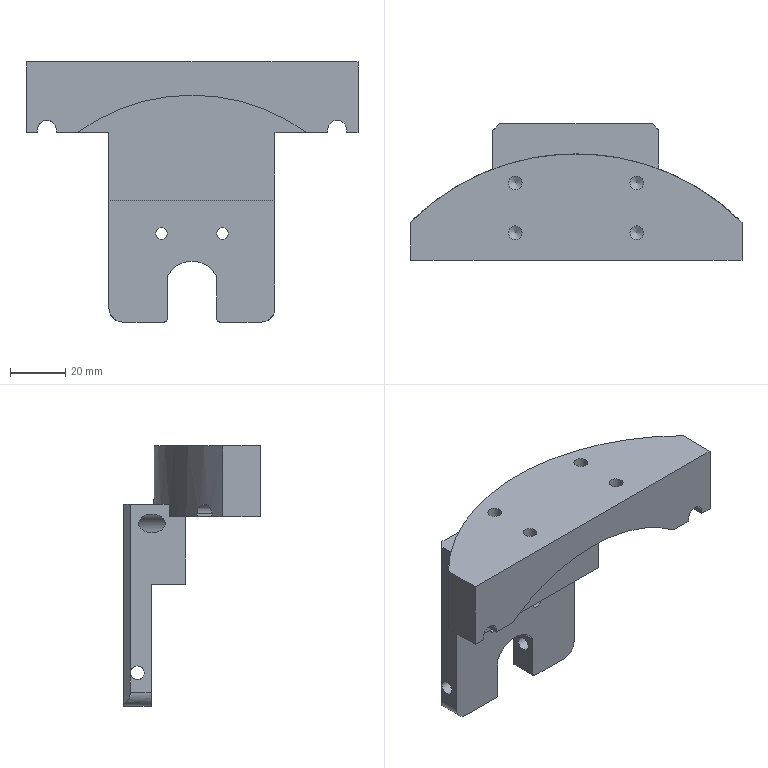Part | NX | features BREP 1 | 1 solid | 48 faces | box 120 x 49.5 x 94 mm | volume 128256 mm3 | plane 25 | cylinder 19 | cone 4 | commonest cylinder face diameters 5 x6 6.8 x4 2 x2 4.2 x2 10 x2 20 x1
STEP:
#1=CARTESIAN_POINT('',(11.,0.,-38.9));
#2=VERTEX_POINT('',#1);
#3=CARTESIAN_POINT('',(11.,0.,-41.));
#4=DIRECTION('',(0.,1.,0.));
#5=DIRECTION('',(0.,0.,1.));
#6=AXIS2_PLACEMENT_3D('',#3,#4,#5);
#7=CIRCLE('',#6,2.1);
#8=EDGE_CURVE('',#2,#2,#7,.T.);
#9=ORIENTED_EDGE('',*,*,#8,.T.);
#10=EDGE_LOOP('',(#9));
#11=FACE_BOUND('',#10,.T.);
#12=CARTESIAN_POINT('',(11.,-10.,-38.9));
#13=VERTEX_POINT('',#12);
#14=CARTESIAN_POINT('',(11.,-10.,-41.));
#15=DIRECTION('',(0.,1.,0.));
#16=DIRECTION('',(0.,0.,1.));
#17=AXIS2_PLACEMENT_3D('',#14,#15,#16);
#18=CIRCLE('',#17,2.1);
#19=EDGE_CURVE('',#13,#13,#18,.T.);
#20=ORIENTED_EDGE('',*,*,#19,.F.);
#21=EDGE_LOOP('',(#20));
#22=FACE_BOUND('',#21,.T.);
#23=CARTESIAN_POINT('',(11.,0.,-41.));
#24=DIRECTION('',(0.,1.,0.));
#25=DIRECTION('',(0.,0.,1.));
#26=AXIS2_PLACEMENT_3D('',#23,#24,#25);
#27=CYLINDRICAL_SURFACE('',#26,2.1);
#28=ADVANCED_FACE('',(#11,#22),#27,.F.);
#29=CARTESIAN_POINT('',(-11.,0.,-38.9));
#30=VERTEX_POINT('',#29);
#31=CARTESIAN_POINT('',(-11.,0.,-41.));
#32=DIRECTION('',(0.,1.,0.));
#33=DIRECTION('',(0.,0.,1.));
#34=AXIS2_PLACEMENT_3D('',#31,#32,#33);
#35=CIRCLE('',#34,2.1);
#36=EDGE_CURVE('',#30,#30,#35,.T.);
#37=ORIENTED_EDGE('',*,*,#36,.T.);
#38=EDGE_LOOP('',(#37));
#39=FACE_BOUND('',#38,.T.);
#40=CARTESIAN_POINT('',(-11.,-10.,-38.9));
#41=VERTEX_POINT('',#40);
#42=CARTESIAN_POINT('',(-11.,-10.,-41.));
#43=DIRECTION('',(0.,1.,0.));
#44=DIRECTION('',(0.,0.,1.));
#45=AXIS2_PLACEMENT_3D('',#42,#43,#44);
#46=CIRCLE('',#45,2.1);
#47=EDGE_CURVE('',#41,#41,#46,.T.);
#48=ORIENTED_EDGE('',*,*,#47,.F.);
#49=EDGE_LOOP('',(#48));
#50=FACE_BOUND('',#49,.T.);
#51=CARTESIAN_POINT('',(-11.,0.,-41.));
#52=DIRECTION('',(0.,1.,0.));
#53=DIRECTION('',(0.,0.,1.));
#54=AXIS2_PLACEMENT_3D('',#51,#52,#53);
#55=CYLINDRICAL_SURFACE('',#54,2.1);
#56=ADVANCED_FACE('',(#39,#50),#55,.F.);
#57=CARTESIAN_POINT('',(30.,-5.47,-7.));
#58=VERTEX_POINT('',#57);
#59=CARTESIAN_POINT('',(30.,-15.087,-7.));
#60=VERTEX_POINT('',#59);
#61=CARTESIAN_POINT('',(30.,-5.47,-7.));
#62=CARTESIAN_POINT('',(30.,-5.47,-13.8));
#63=CARTESIAN_POINT('',(30.,-15.087,-13.8));
#64=CARTESIAN_POINT('',(30.,-15.087,-7.));
#65=(BOUNDED_CURVE()B_SPLINE_CURVE(3,(#61,#62,#63,#64),.UNSPECIFIED.,.F.,.F.)B_SPLINE_CURVE_WITH_KNOTS((4,4),(0.,1.),.PIECEWISE_BEZIER_KNOTS.)CURVE()GEOMETRIC_REPRESENTATION_ITEM()RATIONAL_B_SPLINE_CURVE((1.,0.3333,0.3333,1.))REPRESENTATION_ITEM(''));
#66=EDGE_CURVE('',#58,#60,#65,.T.);
#67=ORIENTED_EDGE('',*,*,#66,.F.);
#68=CARTESIAN_POINT('',(30.,-15.087,-7.));
#69=CARTESIAN_POINT('',(30.,-15.087,-0.2));
#70=CARTESIAN_POINT('',(30.,-5.47,-0.2));
#71=CARTESIAN_POINT('',(30.,-5.47,-7.));
#72=(BOUNDED_CURVE()B_SPLINE_CURVE(3,(#68,#69,#70,#71),.UNSPECIFIED.,.F.,.F.)B_SPLINE_CURVE_WITH_KNOTS((4,4),(0.,1.),.PIECEWISE_BEZIER_KNOTS.)CURVE()GEOMETRIC_REPRESENTATION_ITEM()RATIONAL_B_SPLINE_CURVE((1.,0.3333,0.3333,1.))REPRESENTATION_ITEM(''));
#73=EDGE_CURVE('',#60,#58,#72,.T.);
#74=ORIENTED_EDGE('',*,*,#73,.F.);
#75=EDGE_LOOP('',(#67,#74));
#76=FACE_BOUND('',#75,.T.);
#77=CARTESIAN_POINT('',(24.53,0.,-7.));
#78=VERTEX_POINT('',#77);
#79=CARTESIAN_POINT('',(14.913,0.,-7.));
#80=VERTEX_POINT('',#79);
#81=CARTESIAN_POINT('',(24.53,0.,-7.));
#82=CARTESIAN_POINT('',(24.53,0.,-13.8));
#83=CARTESIAN_POINT('',(14.913,0.,-13.8));
#84=CARTESIAN_POINT('',(14.913,0.,-7.));
#85=(BOUNDED_CURVE()B_SPLINE_CURVE(3,(#81,#82,#83,#84),.UNSPECIFIED.,.F.,.F.)B_SPLINE_CURVE_WITH_KNOTS((4,4),(0.,1.),.PIECEWISE_BEZIER_KNOTS.)CURVE()GEOMETRIC_REPRESENTATION_ITEM()RATIONAL_B_SPLINE_CURVE((1.,0.3333,0.3333,1.))REPRESENTATION_ITEM(''));
#86=EDGE_CURVE('',#78,#80,#85,.T.);
#87=ORIENTED_EDGE('',*,*,#86,.T.);
#88=CARTESIAN_POINT('',(14.913,0.,-7.));
#89=CARTESIAN_POINT('',(14.913,0.,-0.2));
#90=CARTESIAN_POINT('',(24.53,0.,-0.2));
#91=CARTESIAN_POINT('',(24.53,0.,-7.));
#92=(BOUNDED_CURVE()B_SPLINE_CURVE(3,(#88,#89,#90,#91),.UNSPECIFIED.,.F.,.F.)B_SPLINE_CURVE_WITH_KNOTS((4,4),(0.,1.),.PIECEWISE_BEZIER_KNOTS.)CURVE()GEOMETRIC_REPRESENTATION_ITEM()RATIONAL_B_SPLINE_CURVE((1.,0.3333,0.3333,1.))REPRESENTATION_ITEM(''));
#93=EDGE_CURVE('',#80,#78,#92,.T.);
#94=ORIENTED_EDGE('',*,*,#93,.T.);
#95=EDGE_LOOP('',(#87,#94));
#96=FACE_BOUND('',#95,.T.);
#97=CARTESIAN_POINT('',(14.898,4.824,-7.));
#98=DIRECTION('',(0.7071,-0.7071,0.));
#99=DIRECTION('',(0.7071,0.7071,0.));
#100=AXIS2_PLACEMENT_3D('',#97,#98,#99);
#101=CYLINDRICAL_SURFACE('',#100,3.4);
#102=ADVANCED_FACE('',(#76,#96),#101,.F.);
#103=CARTESIAN_POINT('',(-30.,-15.087,-7.));
#104=VERTEX_POINT('',#103);
#105=CARTESIAN_POINT('',(-30.,-5.47,-7.));
#106=VERTEX_POINT('',#105);
#107=CARTESIAN_POINT('',(-30.,-15.087,-7.));
#108=CARTESIAN_POINT('',(-30.,-15.087,-13.8));
#109=CARTESIAN_POINT('',(-30.,-5.47,-13.8));
#110=CARTESIAN_POINT('',(-30.,-5.47,-7.));
#111=(BOUNDED_CURVE()B_SPLINE_CURVE(3,(#107,#108,#109,#110),.UNSPECIFIED.,.F.,.F.)B_SPLINE_CURVE_WITH_KNOTS((4,4),(0.,1.),.PIECEWISE_BEZIER_KNOTS.)CURVE()GEOMETRIC_REPRESENTATION_ITEM()RATIONAL_B_SPLINE_CURVE((1.,0.3333,0.3333,1.))REPRESENTATION_ITEM(''));
#112=EDGE_CURVE('',#104,#106,#111,.T.);
#113=ORIENTED_EDGE('',*,*,#112,.F.);
#114=CARTESIAN_POINT('',(-30.,-5.47,-7.));
#115=CARTESIAN_POINT('',(-30.,-5.47,-0.2));
#116=CARTESIAN_POINT('',(-30.,-15.087,-0.2));
#117=CARTESIAN_POINT('',(-30.,-15.087,-7.));
#118=(BOUNDED_CURVE()B_SPLINE_CURVE(3,(#114,#115,#116,#117),.UNSPECIFIED.,.F.,.F.)B_SPLINE_CURVE_WITH_KNOTS((4,4),(0.,1.),.PIECEWISE_BEZIER_KNOTS.)CURVE()GEOMETRIC_REPRESENTATION_ITEM()RATIONAL_B_SPLINE_CURVE((1.,0.3333,0.3333,1.))REPRESENTATION_ITEM(''));
#119=EDGE_CURVE('',#106,#104,#118,.T.);
#120=ORIENTED_EDGE('',*,*,#119,.F.);
#121=EDGE_LOOP('',(#113,#120));
#122=FACE_BOUND('',#121,.T.);
#123=CARTESIAN_POINT('',(-24.53,0.,-7.));
#124=VERTEX_POINT('',#123);
#125=CARTESIAN_POINT('',(-14.913,0.,-7.));
#126=VERTEX_POINT('',#125);
#127=CARTESIAN_POINT('',(-24.53,0.,-7.));
#128=CARTESIAN_POINT('',(-24.53,0.,-13.8));
#129=CARTESIAN_POINT('',(-14.913,0.,-13.8));
#130=CARTESIAN_POINT('',(-14.913,0.,-7.));
#131=(BOUNDED_CURVE()B_SPLINE_CURVE(3,(#127,#128,#129,#130),.UNSPECIFIED.,.F.,.F.)B_SPLINE_CURVE_WITH_KNOTS((4,4),(0.,1.),.PIECEWISE_BEZIER_KNOTS.)CURVE()GEOMETRIC_REPRESENTATION_ITEM()RATIONAL_B_SPLINE_CURVE((1.,0.3333,0.3333,1.))REPRESENTATION_ITEM(''));
#132=EDGE_CURVE('',#124,#126,#131,.T.);
#133=ORIENTED_EDGE('',*,*,#132,.F.);
#134=CARTESIAN_POINT('',(-14.913,0.,-7.));
#135=CARTESIAN_POINT('',(-14.913,0.,-0.2));
#136=CARTESIAN_POINT('',(-24.53,0.,-0.2));
#137=CARTESIAN_POINT('',(-24.53,0.,-7.));
#138=(BOUNDED_CURVE()B_SPLINE_CURVE(3,(#134,#135,#136,#137),.UNSPECIFIED.,.F.,.F.)B_SPLINE_CURVE_WITH_KNOTS((4,4),(0.,1.),.PIECEWISE_BEZIER_KNOTS.)CURVE()GEOMETRIC_REPRESENTATION_ITEM()RATIONAL_B_SPLINE_CURVE((1.,0.3333,0.3333,1.))REPRESENTATION_ITEM(''));
#139=EDGE_CURVE('',#126,#124,#138,.T.);
#140=ORIENTED_EDGE('',*,*,#139,.F.);
#141=EDGE_LOOP('',(#133,#140));
#142=FACE_BOUND('',#141,.T.);
#143=CARTESIAN_POINT('',(-14.898,4.824,-7.));
#144=DIRECTION('',(-0.7071,-0.7071,0.));
#145=DIRECTION('',(0.7071,-0.7071,0.));
#146=AXIS2_PLACEMENT_3D('',#143,#144,#145);
#147=CYLINDRICAL_SURFACE('',#146,3.4);
#148=ADVANCED_FACE('',(#122,#142),#147,.F.);
#149=CARTESIAN_POINT('',(24.5,-39.5,21.));
#150=VERTEX_POINT('',#149);
#151=CARTESIAN_POINT('',(22.,-39.5,21.));
#152=DIRECTION('',(0.,0.,1.));
#153=DIRECTION('',(1.,0.,0.));
#154=AXIS2_PLACEMENT_3D('',#151,#152,#153);
#155=CIRCLE('',#154,2.5);
#156=EDGE_CURVE('',#150,#150,#155,.T.);
#157=ORIENTED_EDGE('',*,*,#156,.T.);
#158=EDGE_LOOP('',(#157));
#159=FACE_BOUND('',#158,.T.);
#160=CARTESIAN_POINT('',(24.5,-39.5,9.));
#161=VERTEX_POINT('',#160);
#162=CARTESIAN_POINT('',(22.,-39.5,9.));
#163=DIRECTION('',(0.,0.,1.));
#164=DIRECTION('',(1.,0.,0.));
#165=AXIS2_PLACEMENT_3D('',#162,#163,#164);
#166=CIRCLE('',#165,2.5);
#167=EDGE_CURVE('',#161,#161,#166,.T.);
#168=ORIENTED_EDGE('',*,*,#167,.F.);
#169=EDGE_LOOP('',(#168));
#170=FACE_BOUND('',#169,.T.);
#171=CARTESIAN_POINT('',(22.,-39.5,21.));
#172=DIRECTION('',(0.,0.,1.));
#173=DIRECTION('',(1.,0.,0.));
#174=AXIS2_PLACEMENT_3D('',#171,#172,#173);
#175=CYLINDRICAL_SURFACE('',#174,2.5);
#176=ADVANCED_FACE('',(#159,#170),#175,.F.);
#177=ORIENTED_EDGE('',*,*,#167,.T.);
#178=EDGE_LOOP('',(#177));
#179=FACE_BOUND('',#178,.T.);
#180=CARTESIAN_POINT('',(22.,-39.5,7.498));
#181=VERTEX_POINT('',#180);
#182=VERTEX_LOOP('',#181);
#183=FACE_BOUND('',#182,.T.);
#184=CARTESIAN_POINT('',(22.,-39.5,9.));
#185=DIRECTION('',(0.,0.,1.));
#186=DIRECTION('',(1.,0.,0.));
#187=AXIS2_PLACEMENT_3D('',#184,#185,#186);
#188=CONICAL_SURFACE('',#187,2.5,1.03);
#189=ADVANCED_FACE('',(#179,#183),#188,.F.);
#190=CARTESIAN_POINT('',(24.5,-21.5,21.));
#191=VERTEX_POINT('',#190);
#192=CARTESIAN_POINT('',(22.,-21.5,21.));
#193=DIRECTION('',(0.,0.,1.));
#194=DIRECTION('',(1.,0.,0.));
#195=AXIS2_PLACEMENT_3D('',#192,#193,#194);
#196=CIRCLE('',#195,2.5);
#197=EDGE_CURVE('',#191,#191,#196,.T.);
#198=ORIENTED_EDGE('',*,*,#197,.T.);
#199=EDGE_LOOP('',(#198));
#200=FACE_BOUND('',#199,.T.);
#201=CARTESIAN_POINT('',(24.5,-21.5,9.));
#202=VERTEX_POINT('',#201);
#203=CARTESIAN_POINT('',(22.,-21.5,9.));
#204=DIRECTION('',(0.,0.,1.));
#205=DIRECTION('',(1.,0.,0.));
#206=AXIS2_PLACEMENT_3D('',#203,#204,#205);
#207=CIRCLE('',#206,2.5);
#208=EDGE_CURVE('',#202,#202,#207,.T.);
#209=ORIENTED_EDGE('',*,*,#208,.F.);
#210=EDGE_LOOP('',(#209));
#211=FACE_BOUND('',#210,.T.);
#212=CARTESIAN_POINT('',(22.,-21.5,21.));
#213=DIRECTION('',(0.,0.,1.));
#214=DIRECTION('',(1.,0.,0.));
#215=AXIS2_PLACEMENT_3D('',#212,#213,#214);
#216=CYLINDRICAL_SURFACE('',#215,2.5);
#217=ADVANCED_FACE('',(#200,#211),#216,.F.);
#218=ORIENTED_EDGE('',*,*,#208,.T.);
#219=EDGE_LOOP('',(#218));
#220=FACE_BOUND('',#219,.T.);
#221=CARTESIAN_POINT('',(22.,-21.5,7.498));
#222=VERTEX_POINT('',#221);
#223=VERTEX_LOOP('',#222);
#224=FACE_BOUND('',#223,.T.);
#225=CARTESIAN_POINT('',(22.,-21.5,9.));
#226=DIRECTION('',(0.,0.,1.));
#227=DIRECTION('',(1.,0.,0.));
#228=AXIS2_PLACEMENT_3D('',#225,#226,#227);
#229=CONICAL_SURFACE('',#228,2.5,1.03);
#230=ADVANCED_FACE('',(#220,#224),#229,.F.);
#231=CARTESIAN_POINT('',(-19.5,-21.5,21.));
#232=VERTEX_POINT('',#231);
#233=CARTESIAN_POINT('',(-22.,-21.5,21.));
#234=DIRECTION('',(0.,0.,1.));
#235=DIRECTION('',(1.,0.,0.));
#236=AXIS2_PLACEMENT_3D('',#233,#234,#235);
#237=CIRCLE('',#236,2.5);
#238=EDGE_CURVE('',#232,#232,#237,.T.);
#239=ORIENTED_EDGE('',*,*,#238,.T.);
#240=EDGE_LOOP('',(#239));
#241=FACE_BOUND('',#240,.T.);
#242=CARTESIAN_POINT('',(-19.5,-21.5,9.));
#243=VERTEX_POINT('',#242);
#244=CARTESIAN_POINT('',(-22.,-21.5,9.));
#245=DIRECTION('',(0.,0.,1.));
#246=DIRECTION('',(1.,0.,0.));
#247=AXIS2_PLACEMENT_3D('',#244,#245,#246);
#248=CIRCLE('',#247,2.5);
#249=EDGE_CURVE('',#243,#243,#248,.T.);
#250=ORIENTED_EDGE('',*,*,#249,.F.);
#251=EDGE_LOOP('',(#250));
#252=FACE_BOUND('',#251,.T.);
#253=CARTESIAN_POINT('',(-22.,-21.5,21.));
#254=DIRECTION('',(0.,0.,1.));
#255=DIRECTION('',(1.,0.,0.));
#256=AXIS2_PLACEMENT_3D('',#253,#254,#255);
#257=CYLINDRICAL_SURFACE('',#256,2.5);
#258=ADVANCED_FACE('',(#241,#252),#257,.F.);
#259=ORIENTED_EDGE('',*,*,#249,.T.);
#260=EDGE_LOOP('',(#259));
#261=FACE_BOUND('',#260,.T.);
#262=CARTESIAN_POINT('',(-22.,-21.5,7.498));
#263=VERTEX_POINT('',#262);
#264=VERTEX_LOOP('',#263);
#265=FACE_BOUND('',#264,.T.);
#266=CARTESIAN_POINT('',(-22.,-21.5,9.));
#267=DIRECTION('',(0.,0.,1.));
#268=DIRECTION('',(1.,0.,0.));
#269=AXIS2_PLACEMENT_3D('',#266,#267,#268);
#270=CONICAL_SURFACE('',#269,2.5,1.03);
#271=ADVANCED_FACE('',(#261,#265),#270,.F.);
#272=CARTESIAN_POINT('',(-19.5,-39.5,21.));
#273=VERTEX_POINT('',#272);
#274=CARTESIAN_POINT('',(-22.,-39.5,21.));
#275=DIRECTION('',(0.,0.,1.));
#276=DIRECTION('',(1.,0.,0.));
#277=AXIS2_PLACEMENT_3D('',#274,#275,#276);
#278=CIRCLE('',#277,2.5);
#279=EDGE_CURVE('',#273,#273,#278,.T.);
#280=ORIENTED_EDGE('',*,*,#279,.T.);
#281=EDGE_LOOP('',(#280));
#282=FACE_BOUND('',#281,.T.);
#283=CARTESIAN_POINT('',(-19.5,-39.5,9.));
#284=VERTEX_POINT('',#283);
#285=CARTESIAN_POINT('',(-22.,-39.5,9.));
#286=DIRECTION('',(0.,0.,1.));
#287=DIRECTION('',(1.,0.,0.));
#288=AXIS2_PLACEMENT_3D('',#285,#286,#287);
#289=CIRCLE('',#288,2.5);
#290=EDGE_CURVE('',#284,#284,#289,.T.);
#291=ORIENTED_EDGE('',*,*,#290,.F.);
#292=EDGE_LOOP('',(#291));
#293=FACE_BOUND('',#292,.T.);
#294=CARTESIAN_POINT('',(-22.,-39.5,21.));
#295=DIRECTION('',(0.,0.,1.));
#296=DIRECTION('',(1.,0.,0.));
#297=AXIS2_PLACEMENT_3D('',#294,#295,#296);
#298=CYLINDRICAL_SURFACE('',#297,2.5);
#299=ADVANCED_FACE('',(#282,#293),#298,.F.);
#300=ORIENTED_EDGE('',*,*,#290,.T.);
#301=EDGE_LOOP('',(#300));
#302=FACE_BOUND('',#301,.T.);
#303=CARTESIAN_POINT('',(-22.,-39.5,7.498));
#304=VERTEX_POINT('',#303);
#305=VERTEX_LOOP('',#304);
#306=FACE_BOUND('',#305,.T.);
#307=CARTESIAN_POINT('',(-22.,-39.5,9.));
#308=DIRECTION('',(0.,0.,1.));
#309=DIRECTION('',(1.,0.,0.));
#310=AXIS2_PLACEMENT_3D('',#307,#308,#309);
#311=CONICAL_SURFACE('',#310,2.5,1.03);
#312=ADVANCED_FACE('',(#302,#306),#311,.F.);
#313=CARTESIAN_POINT('',(30.,-2.5,-61.));
#314=VERTEX_POINT('',#313);
#315=CARTESIAN_POINT('',(30.,-5.,-61.));
#316=DIRECTION('',(1.,0.,0.));
#317=DIRECTION('',(0.,0.,-1.));
#318=AXIS2_PLACEMENT_3D('',#315,#316,#317);
#319=CIRCLE('',#318,2.5);
#320=EDGE_CURVE('',#314,#314,#319,.T.);
#321=ORIENTED_EDGE('',*,*,#320,.T.);
#322=EDGE_LOOP('',(#321));
#323=FACE_BOUND('',#322,.T.);
#324=CARTESIAN_POINT('',(9.,-5.,-63.5));
#325=VERTEX_POINT('',#324);
#326=CARTESIAN_POINT('',(9.,-5.,-61.));
#327=DIRECTION('',(1.,0.,0.));
#328=DIRECTION('',(0.,0.,-1.));
#329=AXIS2_PLACEMENT_3D('',#326,#327,#328);
#330=CIRCLE('',#329,2.5);
#331=EDGE_CURVE('',#325,#325,#330,.T.);
#332=ORIENTED_EDGE('',*,*,#331,.F.);
#333=EDGE_LOOP('',(#332));
#334=FACE_BOUND('',#333,.T.);
#335=CARTESIAN_POINT('',(30.,-5.,-61.));
#336=DIRECTION('',(1.,0.,0.));
#337=DIRECTION('',(0.,0.,-1.));
#338=AXIS2_PLACEMENT_3D('',#335,#336,#337);
#339=CYLINDRICAL_SURFACE('',#338,2.5);
#340=ADVANCED_FACE('',(#323,#334),#339,.F.);
#341=CARTESIAN_POINT('',(-30.,-2.5,-61.));
#342=VERTEX_POINT('',#341);
#343=CARTESIAN_POINT('',(-30.,-5.,-61.));
#344=DIRECTION('',(-1.,0.,0.));
#345=DIRECTION('',(0.,0.,1.));
#346=AXIS2_PLACEMENT_3D('',#343,#344,#345);
#347=CIRCLE('',#346,2.5);
#348=EDGE_CURVE('',#342,#342,#347,.T.);
#349=ORIENTED_EDGE('',*,*,#348,.T.);
#350=EDGE_LOOP('',(#349));
#351=FACE_BOUND('',#350,.T.);
#352=CARTESIAN_POINT('',(-9.,-5.,-58.5));
#353=VERTEX_POINT('',#352);
#354=CARTESIAN_POINT('',(-9.,-5.,-61.));
#355=DIRECTION('',(-1.,0.,0.));
#356=DIRECTION('',(0.,0.,1.));
#357=AXIS2_PLACEMENT_3D('',#354,#355,#356);
#358=CIRCLE('',#357,2.5);
#359=EDGE_CURVE('',#353,#353,#358,.T.);
#360=ORIENTED_EDGE('',*,*,#359,.F.);
#361=EDGE_LOOP('',(#360));
#362=FACE_BOUND('',#361,.T.);
#363=CARTESIAN_POINT('',(-30.,-5.,-61.));
#364=DIRECTION('',(-1.,0.,0.));
#365=DIRECTION('',(0.,0.,1.));
#366=AXIS2_PLACEMENT_3D('',#363,#364,#365);
#367=CYLINDRICAL_SURFACE('',#366,2.5);
#368=ADVANCED_FACE('',(#351,#362),#367,.F.);
#369=ORIENTED_EDGE('',*,*,#8,.F.);
#370=EDGE_LOOP('',(#369));
#371=FACE_BOUND('',#370,.T.);
#372=ORIENTED_EDGE('',*,*,#36,.F.);
#373=EDGE_LOOP('',(#372));
#374=FACE_BOUND('',#373,.T.);
#375=ORIENTED_EDGE('',*,*,#139,.T.);
#376=ORIENTED_EDGE('',*,*,#132,.T.);
#377=EDGE_LOOP('',(#375,#376));
#378=FACE_BOUND('',#377,.T.);
#379=CARTESIAN_POINT('',(25.,0.,-73.));
#380=VERTEX_POINT('',#379);
#381=CARTESIAN_POINT('',(10.,0.,-73.));
#382=VERTEX_POINT('',#381);
#383=CARTESIAN_POINT('',(30.,0.,-73.));
#384=DIRECTION('',(-1.,0.,0.));
#385=VECTOR('',#384,1000.);
#386=LINE('',#383,#385);
#387=EDGE_CURVE('',#380,#382,#386,.T.);
#388=ORIENTED_EDGE('',*,*,#387,.T.);
#389=CARTESIAN_POINT('',(9.,0.,-72.));
#390=VERTEX_POINT('',#389);
#391=CARTESIAN_POINT('',(10.,0.,-72.));
#392=DIRECTION('',(0.,1.,0.));
#393=DIRECTION('',(0.,0.,-1.));
#394=AXIS2_PLACEMENT_3D('',#391,#392,#393);
#395=CIRCLE('',#394,1.);
#396=EDGE_CURVE('',#382,#390,#395,.T.);
#397=ORIENTED_EDGE('',*,*,#396,.T.);
#398=CARTESIAN_POINT('',(9.,0.,-56.641));
#399=VERTEX_POINT('',#398);
#400=CARTESIAN_POINT('',(9.,0.,-73.));
#401=DIRECTION('',(0.,0.,1.));
#402=VECTOR('',#401,1000.);
#403=LINE('',#400,#402);
#404=EDGE_CURVE('',#390,#399,#403,.T.);
#405=ORIENTED_EDGE('',*,*,#404,.T.);
#406=CARTESIAN_POINT('',(-9.,0.,-56.641));
#407=VERTEX_POINT('',#406);
#408=CARTESIAN_POINT('',(0.,0.,-61.));
#409=DIRECTION('',(0.,-1.,0.));
#410=DIRECTION('',(0.,0.,-1.));
#411=AXIS2_PLACEMENT_3D('',#408,#409,#410);
#412=CIRCLE('',#411,10.);
#413=EDGE_CURVE('',#399,#407,#412,.T.);
#414=ORIENTED_EDGE('',*,*,#413,.T.);
#415=CARTESIAN_POINT('',(-9.,0.,-72.));
#416=VERTEX_POINT('',#415);
#417=CARTESIAN_POINT('',(-9.,0.,-73.));
#418=DIRECTION('',(0.,0.,-1.));
#419=VECTOR('',#418,1000.);
#420=LINE('',#417,#419);
#421=EDGE_CURVE('',#407,#416,#420,.T.);
#422=ORIENTED_EDGE('',*,*,#421,.T.);
#423=CARTESIAN_POINT('',(-10.,0.,-73.));
#424=VERTEX_POINT('',#423);
#425=CARTESIAN_POINT('',(-10.,0.,-72.));
#426=DIRECTION('',(0.,1.,0.));
#427=DIRECTION('',(0.,0.,-1.));
#428=AXIS2_PLACEMENT_3D('',#425,#426,#427);
#429=CIRCLE('',#428,1.);
#430=EDGE_CURVE('',#416,#424,#429,.T.);
#431=ORIENTED_EDGE('',*,*,#430,.T.);
#432=CARTESIAN_POINT('',(-25.,0.,-73.));
#433=VERTEX_POINT('',#432);
#434=CARTESIAN_POINT('',(30.,0.,-73.));
#435=DIRECTION('',(-1.,0.,0.));
#436=VECTOR('',#435,1000.);
#437=LINE('',#434,#436);
#438=EDGE_CURVE('',#424,#433,#437,.T.);
#439=ORIENTED_EDGE('',*,*,#438,.T.);
#440=CARTESIAN_POINT('',(-27.5,0.,-72.33));
#441=VERTEX_POINT('',#440);
#442=CARTESIAN_POINT('',(-25.,0.,-68.));
#443=DIRECTION('',(0.,1.,0.));
#444=DIRECTION('',(0.,0.,-1.));
#445=AXIS2_PLACEMENT_3D('',#442,#443,#444);
#446=CIRCLE('',#445,5.);
#447=EDGE_CURVE('',#433,#441,#446,.T.);
#448=ORIENTED_EDGE('',*,*,#447,.T.);
#449=CARTESIAN_POINT('',(-27.5,0.,0.));
#450=VERTEX_POINT('',#449);
#451=CARTESIAN_POINT('',(-27.5,0.,-73.));
#452=DIRECTION('',(0.,0.,1.));
#453=VECTOR('',#452,1000.);
#454=LINE('',#451,#453);
#455=EDGE_CURVE('',#441,#450,#454,.T.);
#456=ORIENTED_EDGE('',*,*,#455,.T.);
#457=CARTESIAN_POINT('',(27.5,0.,0.));
#458=VERTEX_POINT('',#457);
#459=CARTESIAN_POINT('',(30.,0.,0.));
#460=DIRECTION('',(-1.,0.,0.));
#461=VECTOR('',#460,1000.);
#462=LINE('',#459,#461);
#463=EDGE_CURVE('',#458,#450,#462,.T.);
#464=ORIENTED_EDGE('',*,*,#463,.F.);
#465=CARTESIAN_POINT('',(27.5,0.,-72.33));
#466=VERTEX_POINT('',#465);
#467=CARTESIAN_POINT('',(27.5,0.,-73.));
#468=DIRECTION('',(0.,0.,-1.));
#469=VECTOR('',#468,1000.);
#470=LINE('',#467,#469);
#471=EDGE_CURVE('',#458,#466,#470,.T.);
#472=ORIENTED_EDGE('',*,*,#471,.T.);
#473=CARTESIAN_POINT('',(25.,0.,-68.));
#474=DIRECTION('',(0.,1.,0.));
#475=DIRECTION('',(0.,0.,-1.));
#476=AXIS2_PLACEMENT_3D('',#473,#474,#475);
#477=CIRCLE('',#476,5.);
#478=EDGE_CURVE('',#466,#380,#477,.T.);
#479=ORIENTED_EDGE('',*,*,#478,.T.);
#480=EDGE_LOOP('',(#388,#397,#405,#414,#422,#431,#439,#448,#456,#464,#472,#479));
#481=FACE_BOUND('',#480,.T.);
#482=ORIENTED_EDGE('',*,*,#86,.F.);
#483=ORIENTED_EDGE('',*,*,#93,.F.);
#484=EDGE_LOOP('',(#482,#483));
#485=FACE_BOUND('',#484,.T.);
#486=CARTESIAN_POINT('',(30.,0.,-73.));
#487=DIRECTION('',(0.,-1.,0.));
#488=DIRECTION('',(0.,0.,-1.));
#489=AXIS2_PLACEMENT_3D('',#486,#487,#488);
#490=PLANE('',#489);
#491=ADVANCED_FACE('',(#371,#374,#378,#481,#485),#490,.F.);
#492=CARTESIAN_POINT('',(30.,-2.5,-68.));
#493=VERTEX_POINT('',#492);
#494=CARTESIAN_POINT('',(30.,-2.5,0.));
#495=DIRECTION('',(0.,0.,1.));
#496=VECTOR('',#495,1000.);
#497=LINE('',#494,#496);
#498=EDGE_CURVE('',#493,#314,#497,.T.);
#499=ORIENTED_EDGE('',*,*,#498,.T.);
#500=ORIENTED_EDGE('',*,*,#320,.F.);
#501=CARTESIAN_POINT('',(30.,-2.5,0.));
#502=VERTEX_POINT('',#501);
#503=CARTESIAN_POINT('',(30.,-2.5,0.));
#504=DIRECTION('',(0.,0.,1.));
#505=VECTOR('',#504,1000.);
#506=LINE('',#503,#505);
#507=EDGE_CURVE('',#314,#502,#506,.T.);
#508=ORIENTED_EDGE('',*,*,#507,.T.);
#509=CARTESIAN_POINT('',(30.,-16.47,0.));
#510=VERTEX_POINT('',#509);
#511=CARTESIAN_POINT('',(30.,0.,0.));
#512=DIRECTION('',(0.,-1.,0.));
#513=VECTOR('',#512,1000.);
#514=LINE('',#511,#513);
#515=EDGE_CURVE('',#502,#510,#514,.T.);
#516=ORIENTED_EDGE('',*,*,#515,.T.);
#517=CARTESIAN_POINT('',(30.,-16.47,-4.5));
#518=VERTEX_POINT('',#517);
#519=CARTESIAN_POINT('',(30.,-16.47,-4.));
#520=DIRECTION('',(0.,0.,1.));
#521=VECTOR('',#520,1000.);
#522=LINE('',#519,#521);
#523=EDGE_CURVE('',#518,#510,#522,.T.);
#524=ORIENTED_EDGE('',*,*,#523,.F.);
#525=CARTESIAN_POINT('',(30.,-22.5,-4.5));
#526=VERTEX_POINT('',#525);
#527=CARTESIAN_POINT('',(30.,0.,-4.5));
#528=DIRECTION('',(0.,1.,0.));
#529=VECTOR('',#528,1000.);
#530=LINE('',#527,#529);
#531=EDGE_CURVE('',#526,#518,#530,.T.);
#532=ORIENTED_EDGE('',*,*,#531,.F.);
#533=CARTESIAN_POINT('',(30.,-22.5,-29.));
#534=VERTEX_POINT('',#533);
#535=CARTESIAN_POINT('',(30.,-22.5,0.));
#536=DIRECTION('',(0.,0.,-1.));
#537=VECTOR('',#536,1000.);
#538=LINE('',#535,#537);
#539=EDGE_CURVE('',#526,#534,#538,.T.);
#540=ORIENTED_EDGE('',*,*,#539,.T.);
#541=CARTESIAN_POINT('',(30.,-10.,-29.));
#542=VERTEX_POINT('',#541);
#543=CARTESIAN_POINT('',(30.,-22.5,-29.));
#544=DIRECTION('',(0.,1.,0.));
#545=VECTOR('',#544,1000.);
#546=LINE('',#543,#545);
#547=EDGE_CURVE('',#534,#542,#546,.T.);
#548=ORIENTED_EDGE('',*,*,#547,.T.);
#549=CARTESIAN_POINT('',(30.,-10.,-68.));
#550=VERTEX_POINT('',#549);
#551=CARTESIAN_POINT('',(30.,-10.,-29.));
#552=DIRECTION('',(0.,0.,-1.));
#553=VECTOR('',#552,1000.);
#554=LINE('',#551,#553);
#555=EDGE_CURVE('',#542,#550,#554,.T.);
#556=ORIENTED_EDGE('',*,*,#555,.T.);
#557=CARTESIAN_POINT('',(30.,-2.5,-68.));
#558=DIRECTION('',(0.,1.,0.));
#559=VECTOR('',#558,1000.);
#560=LINE('',#557,#559);
#561=EDGE_CURVE('',#550,#493,#560,.T.);
#562=ORIENTED_EDGE('',*,*,#561,.T.);
#563=EDGE_LOOP('',(#499,#500,#508,#516,#524,#532,#540,#548,#556,#562));
#564=FACE_BOUND('',#563,.T.);
#565=ORIENTED_EDGE('',*,*,#66,.T.);
#566=ORIENTED_EDGE('',*,*,#73,.T.);
#567=EDGE_LOOP('',(#565,#566));
#568=FACE_BOUND('',#567,.T.);
#569=CARTESIAN_POINT('',(30.,0.,0.));
#570=DIRECTION('',(1.,0.,0.));
#571=DIRECTION('',(0.,0.,-1.));
#572=AXIS2_PLACEMENT_3D('',#569,#570,#571);
#573=PLANE('',#572);
#574=ADVANCED_FACE('',(#564,#568),#573,.T.);
#575=CARTESIAN_POINT('',(-49.1,-26.616,-4.5));
#576=VERTEX_POINT('',#575);
#577=CARTESIAN_POINT('',(-49.1,-49.5,-4.5));
#578=VERTEX_POINT('',#577);
#579=CARTESIAN_POINT('',(-49.1,-96.,-4.5));
#580=DIRECTION('',(0.,-1.,0.));
#581=VECTOR('',#580,1000.);
#582=LINE('',#579,#581);
#583=EDGE_CURVE('',#576,#578,#582,.T.);
#584=ORIENTED_EDGE('',*,*,#583,.F.);
#585=CARTESIAN_POINT('',(-30.,-16.47,-4.5));
#586=VERTEX_POINT('',#585);
#587=CARTESIAN_POINT('',(0.,-96.,-4.5));
#588=DIRECTION('',(0.,0.,1.));
#589=DIRECTION('',(-1.,0.,0.));
#590=AXIS2_PLACEMENT_3D('',#587,#588,#589);
#591=CIRCLE('',#590,85.);
#592=EDGE_CURVE('',#586,#576,#591,.T.);
#593=ORIENTED_EDGE('',*,*,#592,.F.);
#594=CARTESIAN_POINT('',(-30.,-22.5,-4.5));
#595=VERTEX_POINT('',#594);
#596=CARTESIAN_POINT('',(-30.,0.,-4.5));
#597=DIRECTION('',(0.,1.,0.));
#598=VECTOR('',#597,1000.);
#599=LINE('',#596,#598);
#600=EDGE_CURVE('',#595,#586,#599,.T.);
#601=ORIENTED_EDGE('',*,*,#600,.F.);
#602=CARTESIAN_POINT('',(-41.325,-22.5,-4.5));
#603=VERTEX_POINT('',#602);
#604=CARTESIAN_POINT('',(-41.325,-22.5,-4.5));
#605=DIRECTION('',(1.,0.,0.));
#606=VECTOR('',#605,1000.);
#607=LINE('',#604,#606);
#608=EDGE_CURVE('',#603,#595,#607,.T.);
#609=ORIENTED_EDGE('',*,*,#608,.F.);
#610=CARTESIAN_POINT('',(-41.325,-49.5,-4.5));
#611=VERTEX_POINT('',#610);
#612=CARTESIAN_POINT('',(-41.325,61.245,-4.5));
#613=DIRECTION('',(0.,-1.,0.));
#614=VECTOR('',#613,1000.);
#615=LINE('',#612,#614);
#616=EDGE_CURVE('',#603,#611,#615,.T.);
#617=ORIENTED_EDGE('',*,*,#616,.T.);
#618=CARTESIAN_POINT('',(-60.,-49.5,-4.5));
#619=DIRECTION('',(1.,0.,0.));
#620=VECTOR('',#619,1000.);
#621=LINE('',#618,#620);
#622=EDGE_CURVE('',#578,#611,#621,.T.);
#623=ORIENTED_EDGE('',*,*,#622,.F.);
#624=EDGE_LOOP('',(#584,#593,#601,#609,#617,#623));
#625=FACE_BOUND('',#624,.T.);
#626=CARTESIAN_POINT('',(0.,-96.,-4.5));
#627=DIRECTION('',(0.,0.,-1.));
#628=DIRECTION('',(-1.,0.,0.));
#629=AXIS2_PLACEMENT_3D('',#626,#627,#628);
#630=PLANE('',#629);
#631=ADVANCED_FACE('',(#625),#630,.T.);
#632=CARTESIAN_POINT('',(55.9,-31.967,-4.5));
#633=VERTEX_POINT('',#632);
#634=CARTESIAN_POINT('',(55.9,-49.5,-4.5));
#635=VERTEX_POINT('',#634);
#636=CARTESIAN_POINT('',(55.9,-96.,-4.5));
#637=DIRECTION('',(0.,-1.,0.));
#638=VECTOR('',#637,1000.);
#639=LINE('',#636,#638);
#640=EDGE_CURVE('',#633,#635,#639,.T.);
#641=ORIENTED_EDGE('',*,*,#640,.F.);
#642=CARTESIAN_POINT('',(60.,-35.792,-4.5));
#643=VERTEX_POINT('',#642);
#644=CARTESIAN_POINT('',(0.,-96.,-4.5));
#645=DIRECTION('',(0.,0.,1.));
#646=DIRECTION('',(-1.,0.,0.));
#647=AXIS2_PLACEMENT_3D('',#644,#645,#646);
#648=CIRCLE('',#647,85.);
#649=EDGE_CURVE('',#643,#633,#648,.T.);
#650=ORIENTED_EDGE('',*,*,#649,.F.);
#651=CARTESIAN_POINT('',(60.,-49.5,-4.5));
#652=VERTEX_POINT('',#651);
#653=CARTESIAN_POINT('',(60.,-49.5,-4.5));
#654=DIRECTION('',(0.,1.,0.));
#655=VECTOR('',#654,1000.);
#656=LINE('',#653,#655);
#657=EDGE_CURVE('',#652,#643,#656,.T.);
#658=ORIENTED_EDGE('',*,*,#657,.F.);
#659=CARTESIAN_POINT('',(-60.,-49.5,-4.5));
#660=DIRECTION('',(1.,0.,0.));
#661=VECTOR('',#660,1000.);
#662=LINE('',#659,#661);
#663=EDGE_CURVE('',#635,#652,#662,.T.);
#664=ORIENTED_EDGE('',*,*,#663,.F.);
#665=EDGE_LOOP('',(#641,#650,#658,#664));
#666=FACE_BOUND('',#665,.T.);
#667=CARTESIAN_POINT('',(0.,-96.,-4.5));
#668=DIRECTION('',(0.,0.,-1.));
#669=DIRECTION('',(-1.,0.,0.));
#670=AXIS2_PLACEMENT_3D('',#667,#668,#669);
#671=PLANE('',#670);
#672=ADVANCED_FACE('',(#666),#671,.T.);
#673=ORIENTED_EDGE('',*,*,#112,.T.);
#674=ORIENTED_EDGE('',*,*,#119,.T.);
#675=EDGE_LOOP('',(#673,#674));
#676=FACE_BOUND('',#675,.T.);
#677=CARTESIAN_POINT('',(-30.,-2.5,0.));
#678=VERTEX_POINT('',#677);
#679=CARTESIAN_POINT('',(-30.,-2.5,0.));
#680=DIRECTION('',(0.,0.,-1.));
#681=VECTOR('',#680,1000.);
#682=LINE('',#679,#681);
#683=EDGE_CURVE('',#678,#342,#682,.T.);
#684=ORIENTED_EDGE('',*,*,#683,.T.);
#685=ORIENTED_EDGE('',*,*,#348,.F.);
#686=CARTESIAN_POINT('',(-30.,-2.5,-68.));
#687=VERTEX_POINT('',#686);
#688=CARTESIAN_POINT('',(-30.,-2.5,0.));
#689=DIRECTION('',(0.,0.,-1.));
#690=VECTOR('',#689,1000.);
#691=LINE('',#688,#690);
#692=EDGE_CURVE('',#342,#687,#691,.T.);
#693=ORIENTED_EDGE('',*,*,#692,.T.);
#694=CARTESIAN_POINT('',(-30.,-10.,-68.));
#695=VERTEX_POINT('',#694);
#696=CARTESIAN_POINT('',(-30.,0.,-68.));
#697=DIRECTION('',(0.,-1.,0.));
#698=VECTOR('',#697,1000.);
#699=LINE('',#696,#698);
#700=EDGE_CURVE('',#687,#695,#699,.T.);
#701=ORIENTED_EDGE('',*,*,#700,.T.);
#702=CARTESIAN_POINT('',(-30.,-10.,-29.));
#703=VERTEX_POINT('',#702);
#704=CARTESIAN_POINT('',(-30.,-10.,-29.));
#705=DIRECTION('',(0.,0.,-1.));
#706=VECTOR('',#705,1000.);
#707=LINE('',#704,#706);
#708=EDGE_CURVE('',#703,#695,#707,.T.);
#709=ORIENTED_EDGE('',*,*,#708,.F.);
#710=CARTESIAN_POINT('',(-30.,-22.5,-29.));
#711=VERTEX_POINT('',#710);
#712=CARTESIAN_POINT('',(-30.,-22.5,-29.));
#713=DIRECTION('',(0.,1.,0.));
#714=VECTOR('',#713,1000.);
#715=LINE('',#712,#714);
#716=EDGE_CURVE('',#711,#703,#715,.T.);
#717=ORIENTED_EDGE('',*,*,#716,.F.);
#718=CARTESIAN_POINT('',(-30.,-22.5,0.));
#719=DIRECTION('',(0.,0.,-1.));
#720=VECTOR('',#719,1000.);
#721=LINE('',#718,#720);
#722=EDGE_CURVE('',#595,#711,#721,.T.);
#723=ORIENTED_EDGE('',*,*,#722,.F.);
#724=ORIENTED_EDGE('',*,*,#600,.T.);
#725=CARTESIAN_POINT('',(-30.,-16.47,0.));
#726=VERTEX_POINT('',#725);
#727=CARTESIAN_POINT('',(-30.,-16.47,-4.));
#728=DIRECTION('',(0.,0.,1.));
#729=VECTOR('',#728,1000.);
#730=LINE('',#727,#729);
#731=EDGE_CURVE('',#586,#726,#730,.T.);
#732=ORIENTED_EDGE('',*,*,#731,.T.);
#733=CARTESIAN_POINT('',(-30.,0.,0.));
#734=DIRECTION('',(0.,-1.,0.));
#735=VECTOR('',#734,1000.);
#736=LINE('',#733,#735);
#737=EDGE_CURVE('',#678,#726,#736,.T.);
#738=ORIENTED_EDGE('',*,*,#737,.F.);
#739=EDGE_LOOP('',(#684,#685,#693,#701,#709,#717,#723,#724,#732,#738));
#740=FACE_BOUND('',#739,.T.);
#741=CARTESIAN_POINT('',(-30.,0.,0.));
#742=DIRECTION('',(1.,0.,0.));
#743=DIRECTION('',(0.,0.,-1.));
#744=AXIS2_PLACEMENT_3D('',#741,#742,#743);
#745=PLANE('',#744);
#746=ADVANCED_FACE('',(#676,#740),#745,.F.);
#747=CARTESIAN_POINT('',(49.1,-49.5,-4.5));
#748=VERTEX_POINT('',#747);
#749=CARTESIAN_POINT('',(49.1,-26.616,-4.5));
#750=VERTEX_POINT('',#749);
#751=CARTESIAN_POINT('',(49.1,-96.,-4.5));
#752=DIRECTION('',(0.,1.,0.));
#753=VECTOR('',#752,1000.);
#754=LINE('',#751,#753);
#755=EDGE_CURVE('',#748,#750,#754,.T.);
#756=ORIENTED_EDGE('',*,*,#755,.F.);
#757=CARTESIAN_POINT('',(41.325,-49.5,-4.5));
#758=VERTEX_POINT('',#757);
#759=CARTESIAN_POINT('',(-60.,-49.5,-4.5));
#760=DIRECTION('',(1.,0.,0.));
#761=VECTOR('',#760,1000.);
#762=LINE('',#759,#761);
#763=EDGE_CURVE('',#758,#748,#762,.T.);
#764=ORIENTED_EDGE('',*,*,#763,.F.);
#765=CARTESIAN_POINT('',(41.325,-22.5,-4.5));
#766=VERTEX_POINT('',#765);
#767=CARTESIAN_POINT('',(41.325,61.245,-4.5));
#768=DIRECTION('',(0.,-1.,0.));
#769=VECTOR('',#768,1000.);
#770=LINE('',#767,#769);
#771=EDGE_CURVE('',#766,#758,#770,.T.);
#772=ORIENTED_EDGE('',*,*,#771,.F.);
#773=CARTESIAN_POINT('',(-41.325,-22.5,-4.5));
#774=DIRECTION('',(1.,0.,0.));
#775=VECTOR('',#774,1000.);
#776=LINE('',#773,#775);
#777=EDGE_CURVE('',#526,#766,#776,.T.);
#778=ORIENTED_EDGE('',*,*,#777,.F.);
#779=ORIENTED_EDGE('',*,*,#531,.T.);
#780=CARTESIAN_POINT('',(0.,-96.,-4.5));
#781=DIRECTION('',(0.,0.,1.));
#782=DIRECTION('',(-1.,0.,0.));
#783=AXIS2_PLACEMENT_3D('',#780,#781,#782);
#784=CIRCLE('',#783,85.);
#785=EDGE_CURVE('',#750,#518,#784,.T.);
#786=ORIENTED_EDGE('',*,*,#785,.F.);
#787=EDGE_LOOP('',(#756,#764,#772,#778,#779,#786));
#788=FACE_BOUND('',#787,.T.);
#789=CARTESIAN_POINT('',(0.,-96.,-4.5));
#790=DIRECTION('',(0.,0.,-1.));
#791=DIRECTION('',(-1.,0.,0.));
#792=AXIS2_PLACEMENT_3D('',#789,#790,#791);
#793=PLANE('',#792);
#794=ADVANCED_FACE('',(#788),#793,.T.);
#795=ORIENTED_EDGE('',*,*,#438,.F.);
#796=CARTESIAN_POINT('',(-10.,-10.,-73.));
#797=VERTEX_POINT('',#796);
#798=CARTESIAN_POINT('',(-10.,-10.,-73.));
#799=DIRECTION('',(0.,-1.,0.));
#800=VECTOR('',#799,1000.);
#801=LINE('',#798,#800);
#802=EDGE_CURVE('',#424,#797,#801,.T.);
#803=ORIENTED_EDGE('',*,*,#802,.T.);
#804=CARTESIAN_POINT('',(-25.,-10.,-73.));
#805=VERTEX_POINT('',#804);
#806=CARTESIAN_POINT('',(30.,-10.,-73.));
#807=DIRECTION('',(-1.,0.,0.));
#808=VECTOR('',#807,1000.);
#809=LINE('',#806,#808);
#810=EDGE_CURVE('',#797,#805,#809,.T.);
#811=ORIENTED_EDGE('',*,*,#810,.T.);
#812=CARTESIAN_POINT('',(-25.,-10.,-73.));
#813=DIRECTION('',(0.,1.,0.));
#814=VECTOR('',#813,1000.);
#815=LINE('',#812,#814);
#816=EDGE_CURVE('',#805,#433,#815,.T.);
#817=ORIENTED_EDGE('',*,*,#816,.T.);
#818=EDGE_LOOP('',(#795,#803,#811,#817));
#819=FACE_BOUND('',#818,.T.);
#820=CARTESIAN_POINT('',(30.,-10.,-73.));
#821=DIRECTION('',(0.,0.,1.));
#822=DIRECTION('',(1.,0.,0.));
#823=AXIS2_PLACEMENT_3D('',#820,#821,#822);
#824=PLANE('',#823);
#825=ADVANCED_FACE('',(#819),#824,.F.);
#826=CARTESIAN_POINT('',(-49.1,-26.616,-3.5));
#827=VERTEX_POINT('',#826);
#828=CARTESIAN_POINT('',(-49.1,-26.616,-4.5));
#829=DIRECTION('',(0.,0.,-1.));
#830=VECTOR('',#829,1000.);
#831=LINE('',#828,#830);
#832=EDGE_CURVE('',#827,#576,#831,.T.);
#833=ORIENTED_EDGE('',*,*,#832,.F.);
#834=CARTESIAN_POINT('',(-55.9,-31.967,-3.5));
#835=VERTEX_POINT('',#834);
#836=CARTESIAN_POINT('',(-55.9,-31.967,-3.5));
#837=CARTESIAN_POINT('',(-55.9,-31.967,-2.471));
#838=CARTESIAN_POINT('',(-54.921,-31.108,-0.6534));
#839=CARTESIAN_POINT('',(-52.568,-29.178,0.1619));
#840=CARTESIAN_POINT('',(-50.104,-27.321,-0.5965));
#841=CARTESIAN_POINT('',(-49.1,-26.616,-2.471));
#842=CARTESIAN_POINT('',(-49.1,-26.616,-3.5));
#843=B_SPLINE_CURVE_WITH_KNOTS('',3,(#836,#837,#838,#839,#840,#841,#842),.UNSPECIFIED.,.F.,.F.,(4,1,1,1,4),(0.,0.003035,0.00607,0.009106,0.01214),.UNSPECIFIED.);
#844=EDGE_CURVE('',#835,#827,#843,.T.);
#845=ORIENTED_EDGE('',*,*,#844,.F.);
#846=CARTESIAN_POINT('',(-55.9,-31.967,-4.5));
#847=VERTEX_POINT('',#846);
#848=CARTESIAN_POINT('',(-55.9,-31.967,-4.5));
#849=DIRECTION('',(0.,0.,1.));
#850=VECTOR('',#849,1000.);
#851=LINE('',#848,#850);
#852=EDGE_CURVE('',#847,#835,#851,.T.);
#853=ORIENTED_EDGE('',*,*,#852,.F.);
#854=CARTESIAN_POINT('',(-60.,-35.792,-4.5));
#855=VERTEX_POINT('',#854);
#856=CARTESIAN_POINT('',(0.,-96.,-4.5));
#857=DIRECTION('',(0.,0.,1.));
#858=DIRECTION('',(-1.,0.,0.));
#859=AXIS2_PLACEMENT_3D('',#856,#857,#858);
#860=CIRCLE('',#859,85.);
#861=EDGE_CURVE('',#847,#855,#860,.T.);
#862=ORIENTED_EDGE('',*,*,#861,.T.);
#863=CARTESIAN_POINT('',(-60.,-35.792,21.));
#864=VERTEX_POINT('',#863);
#865=CARTESIAN_POINT('',(-60.,-35.792,-4.5));
#866=DIRECTION('',(0.,0.,1.));
#867=VECTOR('',#866,1000.);
#868=LINE('',#865,#867);
#869=EDGE_CURVE('',#855,#864,#868,.T.);
#870=ORIENTED_EDGE('',*,*,#869,.T.);
#871=CARTESIAN_POINT('',(60.,-35.792,21.));
#872=VERTEX_POINT('',#871);
#873=CARTESIAN_POINT('',(0.,-96.,21.));
#874=DIRECTION('',(0.,0.,1.));
#875=DIRECTION('',(-1.,0.,0.));
#876=AXIS2_PLACEMENT_3D('',#873,#874,#875);
#877=CIRCLE('',#876,85.);
#878=EDGE_CURVE('',#872,#864,#877,.T.);
#879=ORIENTED_EDGE('',*,*,#878,.F.);
#880=CARTESIAN_POINT('',(60.,-35.792,-4.5));
#881=DIRECTION('',(0.,0.,1.));
#882=VECTOR('',#881,1000.);
#883=LINE('',#880,#882);
#884=EDGE_CURVE('',#643,#872,#883,.T.);
#885=ORIENTED_EDGE('',*,*,#884,.F.);
#886=ORIENTED_EDGE('',*,*,#649,.T.);
#887=CARTESIAN_POINT('',(55.9,-31.967,-3.5));
#888=VERTEX_POINT('',#887);
#889=CARTESIAN_POINT('',(55.9,-31.967,-4.5));
#890=DIRECTION('',(0.,0.,-1.));
#891=VECTOR('',#890,1000.);
#892=LINE('',#889,#891);
#893=EDGE_CURVE('',#888,#633,#892,.T.);
#894=ORIENTED_EDGE('',*,*,#893,.F.);
#895=CARTESIAN_POINT('',(49.1,-26.616,-3.5));
#896=VERTEX_POINT('',#895);
#897=CARTESIAN_POINT('',(49.1,-26.616,-3.5));
#898=CARTESIAN_POINT('',(49.1,-26.616,-2.474));
#899=CARTESIAN_POINT('',(50.098,-27.316,-0.5983));
#900=CARTESIAN_POINT('',(52.577,-29.185,0.1608));
#901=CARTESIAN_POINT('',(54.912,-31.101,-0.6475));
#902=CARTESIAN_POINT('',(55.9,-31.967,-2.471));
#903=CARTESIAN_POINT('',(55.9,-31.967,-3.5));
#904=B_SPLINE_CURVE_WITH_KNOTS('',3,(#897,#898,#899,#900,#901,#902,#903),.UNSPECIFIED.,.F.,.F.,(4,1,1,1,4),(0.,0.003031,0.006062,0.009093,0.01212),.UNSPECIFIED.);
#905=EDGE_CURVE('',#896,#888,#904,.T.);
#906=ORIENTED_EDGE('',*,*,#905,.F.);
#907=CARTESIAN_POINT('',(49.1,-26.616,-4.5));
#908=DIRECTION('',(0.,0.,1.));
#909=VECTOR('',#908,1000.);
#910=LINE('',#907,#909);
#911=EDGE_CURVE('',#750,#896,#910,.T.);
#912=ORIENTED_EDGE('',*,*,#911,.F.);
#913=ORIENTED_EDGE('',*,*,#785,.T.);
#914=ORIENTED_EDGE('',*,*,#523,.T.);
#915=CARTESIAN_POINT('',(0.,-96.,0.));
#916=DIRECTION('',(0.,0.,1.));
#917=DIRECTION('',(-1.,0.,0.));
#918=AXIS2_PLACEMENT_3D('',#915,#916,#917);
#919=CIRCLE('',#918,85.);
#920=EDGE_CURVE('',#510,#726,#919,.T.);
#921=ORIENTED_EDGE('',*,*,#920,.T.);
#922=ORIENTED_EDGE('',*,*,#731,.F.);
#923=ORIENTED_EDGE('',*,*,#592,.T.);
#924=EDGE_LOOP('',(#833,#845,#853,#862,#870,#879,#885,#886,#894,#906,#912,#913,#914,#921,#922,#923));
#925=FACE_BOUND('',#924,.T.);
#926=CARTESIAN_POINT('',(0.,-96.,-4.5));
#927=DIRECTION('',(0.,0.,1.));
#928=DIRECTION('',(1.,0.,0.));
#929=AXIS2_PLACEMENT_3D('',#926,#927,#928);
#930=CYLINDRICAL_SURFACE('',#929,85.);
#931=ADVANCED_FACE('',(#925),#930,.T.);
#932=CARTESIAN_POINT('',(-60.,-49.5,21.));
#933=VERTEX_POINT('',#932);
#934=CARTESIAN_POINT('',(-60.,-49.5,21.));
#935=DIRECTION('',(0.,-1.,0.));
#936=VECTOR('',#935,1000.);
#937=LINE('',#934,#936);
#938=EDGE_CURVE('',#864,#933,#937,.T.);
#939=ORIENTED_EDGE('',*,*,#938,.F.);
#940=ORIENTED_EDGE('',*,*,#869,.F.);
#941=CARTESIAN_POINT('',(-60.,-49.5,-4.5));
#942=VERTEX_POINT('',#941);
#943=CARTESIAN_POINT('',(-60.,-49.5,-4.5));
#944=DIRECTION('',(0.,-1.,0.));
#945=VECTOR('',#944,1000.);
#946=LINE('',#943,#945);
#947=EDGE_CURVE('',#855,#942,#946,.T.);
#948=ORIENTED_EDGE('',*,*,#947,.T.);
#949=CARTESIAN_POINT('',(-60.,-49.5,-4.5));
#950=DIRECTION('',(0.,0.,1.));
#951=VECTOR('',#950,1000.);
#952=LINE('',#949,#951);
#953=EDGE_CURVE('',#942,#933,#952,.T.);
#954=ORIENTED_EDGE('',*,*,#953,.T.);
#955=EDGE_LOOP('',(#939,#940,#948,#954));
#956=FACE_BOUND('',#955,.T.);
#957=CARTESIAN_POINT('',(-60.,-49.5,-4.5));
#958=DIRECTION('',(-1.,0.,0.));
#959=DIRECTION('',(0.,0.,1.));
#960=AXIS2_PLACEMENT_3D('',#957,#958,#959);
#961=PLANE('',#960);
#962=ADVANCED_FACE('',(#956),#961,.T.);
#963=CARTESIAN_POINT('',(60.,-49.5,21.));
#964=VERTEX_POINT('',#963);
#965=CARTESIAN_POINT('',(60.,-49.5,21.));
#966=DIRECTION('',(0.,1.,0.));
#967=VECTOR('',#966,1000.);
#968=LINE('',#965,#967);
#969=EDGE_CURVE('',#964,#872,#968,.T.);
#970=ORIENTED_EDGE('',*,*,#969,.F.);
#971=CARTESIAN_POINT('',(60.,-49.5,-4.5));
#972=DIRECTION('',(0.,0.,1.));
#973=VECTOR('',#972,1000.);
#974=LINE('',#971,#973);
#975=EDGE_CURVE('',#652,#964,#974,.T.);
#976=ORIENTED_EDGE('',*,*,#975,.F.);
#977=ORIENTED_EDGE('',*,*,#657,.T.);
#978=ORIENTED_EDGE('',*,*,#884,.T.);
#979=EDGE_LOOP('',(#970,#976,#977,#978));
#980=FACE_BOUND('',#979,.T.);
#981=CARTESIAN_POINT('',(60.,-49.5,-4.5));
#982=DIRECTION('',(1.,0.,0.));
#983=DIRECTION('',(0.,0.,-1.));
#984=AXIS2_PLACEMENT_3D('',#981,#982,#983);
#985=PLANE('',#984);
#986=ADVANCED_FACE('',(#980),#985,.T.);
#987=CARTESIAN_POINT('',(-49.1,-49.5,-3.5));
#988=VERTEX_POINT('',#987);
#989=CARTESIAN_POINT('',(-49.1,-49.5,-3.5));
#990=DIRECTION('',(0.,0.,1.));
#991=VECTOR('',#990,1000.);
#992=LINE('',#989,#991);
#993=EDGE_CURVE('',#578,#988,#992,.T.);
#994=ORIENTED_EDGE('',*,*,#993,.F.);
#995=ORIENTED_EDGE('',*,*,#622,.T.);
#996=CARTESIAN_POINT('',(0.,-49.5,-61.));
#997=DIRECTION('',(0.,-1.,0.));
#998=DIRECTION('',(1.,0.,0.));
#999=AXIS2_PLACEMENT_3D('',#996,#997,#998);
#1000=CIRCLE('',#999,70.);
#1001=EDGE_CURVE('',#758,#611,#1000,.T.);
#1002=ORIENTED_EDGE('',*,*,#1001,.F.);
#1003=ORIENTED_EDGE('',*,*,#763,.T.);
#1004=CARTESIAN_POINT('',(49.1,-49.5,-3.5));
#1005=VERTEX_POINT('',#1004);
#1006=CARTESIAN_POINT('',(49.1,-49.5,-3.5));
#1007=DIRECTION('',(0.,0.,-1.));
#1008=VECTOR('',#1007,1000.);
#1009=LINE('',#1006,#1008);
#1010=EDGE_CURVE('',#1005,#748,#1009,.T.);
#1011=ORIENTED_EDGE('',*,*,#1010,.F.);
#1012=CARTESIAN_POINT('',(55.9,-49.5,-3.5));
#1013=VERTEX_POINT('',#1012);
#1014=CARTESIAN_POINT('',(52.5,-49.5,-3.5));
#1015=DIRECTION('',(0.,-1.,0.));
#1016=DIRECTION('',(-1.,0.,0.));
#1017=AXIS2_PLACEMENT_3D('',#1014,#1015,#1016);
#1018=CIRCLE('',#1017,3.4);
#1019=EDGE_CURVE('',#1013,#1005,#1018,.T.);
#1020=ORIENTED_EDGE('',*,*,#1019,.F.);
#1021=CARTESIAN_POINT('',(55.9,-49.5,-4.5));
#1022=DIRECTION('',(0.,0.,1.));
#1023=VECTOR('',#1022,1000.);
#1024=LINE('',#1021,#1023);
#1025=EDGE_CURVE('',#635,#1013,#1024,.T.);
#1026=ORIENTED_EDGE('',*,*,#1025,.F.);
#1027=ORIENTED_EDGE('',*,*,#663,.T.);
#1028=ORIENTED_EDGE('',*,*,#975,.T.);
#1029=CARTESIAN_POINT('',(-60.,-49.5,21.));
#1030=DIRECTION('',(1.,0.,0.));
#1031=VECTOR('',#1030,1000.);
#1032=LINE('',#1029,#1031);
#1033=EDGE_CURVE('',#933,#964,#1032,.T.);
#1034=ORIENTED_EDGE('',*,*,#1033,.F.);
#1035=ORIENTED_EDGE('',*,*,#953,.F.);
#1036=CARTESIAN_POINT('',(-55.9,-49.5,-4.5));
#1037=VERTEX_POINT('',#1036);
#1038=CARTESIAN_POINT('',(-60.,-49.5,-4.5));
#1039=DIRECTION('',(1.,0.,0.));
#1040=VECTOR('',#1039,1000.);
#1041=LINE('',#1038,#1040);
#1042=EDGE_CURVE('',#942,#1037,#1041,.T.);
#1043=ORIENTED_EDGE('',*,*,#1042,.T.);
#1044=CARTESIAN_POINT('',(-55.9,-49.5,-3.5));
#1045=VERTEX_POINT('',#1044);
#1046=CARTESIAN_POINT('',(-55.9,-49.5,-3.5));
#1047=DIRECTION('',(0.,0.,-1.));
#1048=VECTOR('',#1047,1000.);
#1049=LINE('',#1046,#1048);
#1050=EDGE_CURVE('',#1045,#1037,#1049,.T.);
#1051=ORIENTED_EDGE('',*,*,#1050,.F.);
#1052=CARTESIAN_POINT('',(-52.5,-49.5,-3.5));
#1053=DIRECTION('',(0.,-1.,0.));
#1054=DIRECTION('',(1.,0.,0.));
#1055=AXIS2_PLACEMENT_3D('',#1052,#1053,#1054);
#1056=CIRCLE('',#1055,3.4);
#1057=EDGE_CURVE('',#988,#1045,#1056,.T.);
#1058=ORIENTED_EDGE('',*,*,#1057,.F.);
#1059=EDGE_LOOP('',(#994,#995,#1002,#1003,#1011,#1020,#1026,#1027,#1028,#1034,#1035,#1043,#1051,#1058));
#1060=FACE_BOUND('',#1059,.T.);
#1061=CARTESIAN_POINT('',(-60.,-49.5,-4.5));
#1062=DIRECTION('',(0.,-1.,0.));
#1063=DIRECTION('',(1.,0.,0.));
#1064=AXIS2_PLACEMENT_3D('',#1061,#1062,#1063);
#1065=PLANE('',#1064);
#1066=ADVANCED_FACE('',(#1060),#1065,.T.);
#1067=CARTESIAN_POINT('',(-55.9,-96.,-4.5));
#1068=DIRECTION('',(0.,1.,0.));
#1069=VECTOR('',#1068,1000.);
#1070=LINE('',#1067,#1069);
#1071=EDGE_CURVE('',#1037,#847,#1070,.T.);
#1072=ORIENTED_EDGE('',*,*,#1071,.F.);
#1073=ORIENTED_EDGE('',*,*,#1042,.F.);
#1074=ORIENTED_EDGE('',*,*,#947,.F.);
#1075=ORIENTED_EDGE('',*,*,#861,.F.);
#1076=EDGE_LOOP('',(#1072,#1073,#1074,#1075));
#1077=FACE_BOUND('',#1076,.T.);
#1078=CARTESIAN_POINT('',(0.,-96.,-4.5));
#1079=DIRECTION('',(0.,0.,-1.));
#1080=DIRECTION('',(-1.,0.,0.));
#1081=AXIS2_PLACEMENT_3D('',#1078,#1079,#1080);
#1082=PLANE('',#1081);
#1083=ADVANCED_FACE('',(#1077),#1082,.T.);
#1084=ORIENTED_EDGE('',*,*,#156,.F.);
#1085=EDGE_LOOP('',(#1084));
#1086=FACE_BOUND('',#1085,.T.);
#1087=ORIENTED_EDGE('',*,*,#197,.F.);
#1088=EDGE_LOOP('',(#1087));
#1089=FACE_BOUND('',#1088,.T.);
#1090=ORIENTED_EDGE('',*,*,#238,.F.);
#1091=EDGE_LOOP('',(#1090));
#1092=FACE_BOUND('',#1091,.T.);
#1093=ORIENTED_EDGE('',*,*,#279,.F.);
#1094=EDGE_LOOP('',(#1093));
#1095=FACE_BOUND('',#1094,.T.);
#1096=ORIENTED_EDGE('',*,*,#938,.T.);
#1097=ORIENTED_EDGE('',*,*,#1033,.T.);
#1098=ORIENTED_EDGE('',*,*,#969,.T.);
#1099=ORIENTED_EDGE('',*,*,#878,.T.);
#1100=EDGE_LOOP('',(#1096,#1097,#1098,#1099));
#1101=FACE_BOUND('',#1100,.T.);
#1102=CARTESIAN_POINT('',(0.,-96.,21.));
#1103=DIRECTION('',(0.,0.,-1.));
#1104=DIRECTION('',(-1.,0.,0.));
#1105=AXIS2_PLACEMENT_3D('',#1102,#1103,#1104);
#1106=PLANE('',#1105);
#1107=ADVANCED_FACE('',(#1086,#1089,#1092,#1095,#1101),#1106,.F.);
#1108=CARTESIAN_POINT('',(25.,-10.,-73.));
#1109=VERTEX_POINT('',#1108);
#1110=CARTESIAN_POINT('',(10.,-10.,-73.));
#1111=VERTEX_POINT('',#1110);
#1112=CARTESIAN_POINT('',(30.,-10.,-73.));
#1113=DIRECTION('',(-1.,0.,0.));
#1114=VECTOR('',#1113,1000.);
#1115=LINE('',#1112,#1114);
#1116=EDGE_CURVE('',#1109,#1111,#1115,.T.);
#1117=ORIENTED_EDGE('',*,*,#1116,.T.);
#1118=CARTESIAN_POINT('',(10.,-10.,-73.));
#1119=DIRECTION('',(0.,1.,0.));
#1120=VECTOR('',#1119,1000.);
#1121=LINE('',#1118,#1120);
#1122=EDGE_CURVE('',#1111,#382,#1121,.T.);
#1123=ORIENTED_EDGE('',*,*,#1122,.T.);
#1124=ORIENTED_EDGE('',*,*,#387,.F.);
#1125=CARTESIAN_POINT('',(25.,-10.,-73.));
#1126=DIRECTION('',(0.,-1.,0.));
#1127=VECTOR('',#1126,1000.);
#1128=LINE('',#1125,#1127);
#1129=EDGE_CURVE('',#380,#1109,#1128,.T.);
#1130=ORIENTED_EDGE('',*,*,#1129,.T.);
#1131=EDGE_LOOP('',(#1117,#1123,#1124,#1130));
#1132=FACE_BOUND('',#1131,.T.);
#1133=CARTESIAN_POINT('',(30.,-10.,-73.));
#1134=DIRECTION('',(0.,0.,1.));
#1135=DIRECTION('',(1.,0.,0.));
#1136=AXIS2_PLACEMENT_3D('',#1133,#1134,#1135);
#1137=PLANE('',#1136);
#1138=ADVANCED_FACE('',(#1132),#1137,.F.);
#1139=ORIENTED_EDGE('',*,*,#515,.F.);
#1140=CARTESIAN_POINT('',(30.,-2.5,0.));
#1141=DIRECTION('',(-0.7071,0.7071,0.));
#1142=VECTOR('',#1141,1000.);
#1143=LINE('',#1140,#1142);
#1144=EDGE_CURVE('',#502,#458,#1143,.T.);
#1145=ORIENTED_EDGE('',*,*,#1144,.T.);
#1146=ORIENTED_EDGE('',*,*,#463,.T.);
#1147=CARTESIAN_POINT('',(-27.5,0.,0.));
#1148=DIRECTION('',(-0.7071,-0.7071,0.));
#1149=VECTOR('',#1148,1000.);
#1150=LINE('',#1147,#1149);
#1151=EDGE_CURVE('',#450,#678,#1150,.T.);
#1152=ORIENTED_EDGE('',*,*,#1151,.T.);
#1153=ORIENTED_EDGE('',*,*,#737,.T.);
#1154=ORIENTED_EDGE('',*,*,#920,.F.);
#1155=EDGE_LOOP('',(#1139,#1145,#1146,#1152,#1153,#1154));
#1156=FACE_BOUND('',#1155,.T.);
#1157=CARTESIAN_POINT('',(30.,0.,0.));
#1158=DIRECTION('',(0.,0.,-1.));
#1159=DIRECTION('',(0.,1.,0.));
#1160=AXIS2_PLACEMENT_3D('',#1157,#1158,#1159);
#1161=PLANE('',#1160);
#1162=ADVANCED_FACE('',(#1156),#1161,.F.);
#1163=ORIENTED_EDGE('',*,*,#539,.F.);
#1164=ORIENTED_EDGE('',*,*,#777,.T.);
#1165=CARTESIAN_POINT('',(0.,-22.5,-61.));
#1166=DIRECTION('',(0.,-1.,0.));
#1167=DIRECTION('',(0.,0.,1.));
#1168=AXIS2_PLACEMENT_3D('',#1165,#1166,#1167);
#1169=CIRCLE('',#1168,70.);
#1170=EDGE_CURVE('',#766,#603,#1169,.T.);
#1171=ORIENTED_EDGE('',*,*,#1170,.T.);
#1172=ORIENTED_EDGE('',*,*,#608,.T.);
#1173=ORIENTED_EDGE('',*,*,#722,.T.);
#1174=CARTESIAN_POINT('',(30.,-22.5,-29.));
#1175=DIRECTION('',(-1.,0.,0.));
#1176=VECTOR('',#1175,1000.);
#1177=LINE('',#1174,#1176);
#1178=EDGE_CURVE('',#534,#711,#1177,.T.);
#1179=ORIENTED_EDGE('',*,*,#1178,.F.);
#1180=EDGE_LOOP('',(#1163,#1164,#1171,#1172,#1173,#1179));
#1181=FACE_BOUND('',#1180,.T.);
#1182=CARTESIAN_POINT('',(30.,-22.5,0.));
#1183=DIRECTION('',(0.,1.,0.));
#1184=DIRECTION('',(0.,0.,1.));
#1185=AXIS2_PLACEMENT_3D('',#1182,#1183,#1184);
#1186=PLANE('',#1185);
#1187=ADVANCED_FACE('',(#1181),#1186,.F.);
#1188=ORIENTED_EDGE('',*,*,#716,.T.);
#1189=CARTESIAN_POINT('',(30.,-10.,-29.));
#1190=DIRECTION('',(-1.,0.,0.));
#1191=VECTOR('',#1190,1000.);
#1192=LINE('',#1189,#1191);
#1193=EDGE_CURVE('',#542,#703,#1192,.T.);
#1194=ORIENTED_EDGE('',*,*,#1193,.F.);
#1195=ORIENTED_EDGE('',*,*,#547,.F.);
#1196=ORIENTED_EDGE('',*,*,#1178,.T.);
#1197=EDGE_LOOP('',(#1188,#1194,#1195,#1196));
#1198=FACE_BOUND('',#1197,.T.);
#1199=CARTESIAN_POINT('',(30.,-22.5,-29.));
#1200=DIRECTION('',(0.,0.,1.));
#1201=DIRECTION('',(1.,0.,0.));
#1202=AXIS2_PLACEMENT_3D('',#1199,#1200,#1201);
#1203=PLANE('',#1202);
#1204=ADVANCED_FACE('',(#1198),#1203,.F.);
#1205=ORIENTED_EDGE('',*,*,#19,.T.);
#1206=EDGE_LOOP('',(#1205));
#1207=FACE_BOUND('',#1206,.T.);
#1208=ORIENTED_EDGE('',*,*,#47,.T.);
#1209=EDGE_LOOP('',(#1208));
#1210=FACE_BOUND('',#1209,.T.);
#1211=CARTESIAN_POINT('',(9.,-10.,-72.));
#1212=VERTEX_POINT('',#1211);
#1213=CARTESIAN_POINT('',(9.,-10.,-56.641));
#1214=VERTEX_POINT('',#1213);
#1215=CARTESIAN_POINT('',(9.,-10.,-73.));
#1216=DIRECTION('',(0.,0.,1.));
#1217=VECTOR('',#1216,1000.);
#1218=LINE('',#1215,#1217);
#1219=EDGE_CURVE('',#1212,#1214,#1218,.T.);
#1220=ORIENTED_EDGE('',*,*,#1219,.F.);
#1221=CARTESIAN_POINT('',(10.,-10.,-72.));
#1222=DIRECTION('',(0.,-1.,0.));
#1223=DIRECTION('',(0.,0.,1.));
#1224=AXIS2_PLACEMENT_3D('',#1221,#1222,#1223);
#1225=CIRCLE('',#1224,1.);
#1226=EDGE_CURVE('',#1212,#1111,#1225,.T.);
#1227=ORIENTED_EDGE('',*,*,#1226,.T.);
#1228=ORIENTED_EDGE('',*,*,#1116,.F.);
#1229=CARTESIAN_POINT('',(25.,-10.,-68.));
#1230=DIRECTION('',(0.,-1.,0.));
#1231=DIRECTION('',(0.,0.,1.));
#1232=AXIS2_PLACEMENT_3D('',#1229,#1230,#1231);
#1233=CIRCLE('',#1232,5.);
#1234=EDGE_CURVE('',#1109,#550,#1233,.T.);
#1235=ORIENTED_EDGE('',*,*,#1234,.T.);
#1236=ORIENTED_EDGE('',*,*,#555,.F.);
#1237=ORIENTED_EDGE('',*,*,#1193,.T.);
#1238=ORIENTED_EDGE('',*,*,#708,.T.);
#1239=CARTESIAN_POINT('',(-25.,-10.,-68.));
#1240=DIRECTION('',(0.,-1.,0.));
#1241=DIRECTION('',(0.,0.,1.));
#1242=AXIS2_PLACEMENT_3D('',#1239,#1240,#1241);
#1243=CIRCLE('',#1242,5.);
#1244=EDGE_CURVE('',#695,#805,#1243,.T.);
#1245=ORIENTED_EDGE('',*,*,#1244,.T.);
#1246=ORIENTED_EDGE('',*,*,#810,.F.);
#1247=CARTESIAN_POINT('',(-9.,-10.,-72.));
#1248=VERTEX_POINT('',#1247);
#1249=CARTESIAN_POINT('',(-10.,-10.,-72.));
#1250=DIRECTION('',(0.,-1.,0.));
#1251=DIRECTION('',(0.,0.,1.));
#1252=AXIS2_PLACEMENT_3D('',#1249,#1250,#1251);
#1253=CIRCLE('',#1252,1.);
#1254=EDGE_CURVE('',#797,#1248,#1253,.T.);
#1255=ORIENTED_EDGE('',*,*,#1254,.T.);
#1256=CARTESIAN_POINT('',(-9.,-10.,-56.641));
#1257=VERTEX_POINT('',#1256);
#1258=CARTESIAN_POINT('',(-9.,-10.,-73.));
#1259=DIRECTION('',(0.,0.,-1.));
#1260=VECTOR('',#1259,1000.);
#1261=LINE('',#1258,#1260);
#1262=EDGE_CURVE('',#1257,#1248,#1261,.T.);
#1263=ORIENTED_EDGE('',*,*,#1262,.F.);
#1264=CARTESIAN_POINT('',(0.,-10.,-61.));
#1265=DIRECTION('',(0.,-1.,0.));
#1266=DIRECTION('',(0.,0.,-1.));
#1267=AXIS2_PLACEMENT_3D('',#1264,#1265,#1266);
#1268=CIRCLE('',#1267,10.);
#1269=EDGE_CURVE('',#1214,#1257,#1268,.T.);
#1270=ORIENTED_EDGE('',*,*,#1269,.F.);
#1271=EDGE_LOOP('',(#1220,#1227,#1228,#1235,#1236,#1237,#1238,#1245,#1246,#1255,#1263,#1270));
#1272=FACE_BOUND('',#1271,.T.);
#1273=CARTESIAN_POINT('',(30.,-10.,-29.));
#1274=DIRECTION('',(0.,1.,0.));
#1275=DIRECTION('',(0.,0.,1.));
#1276=AXIS2_PLACEMENT_3D('',#1273,#1274,#1275);
#1277=PLANE('',#1276);
#1278=ADVANCED_FACE('',(#1207,#1210,#1272),#1277,.F.);
#1279=ORIENTED_EDGE('',*,*,#498,.F.);
#1280=CARTESIAN_POINT('',(30.,-2.5,-68.));
#1281=CARTESIAN_POINT('',(30.,-2.5,-69.83));
#1282=CARTESIAN_POINT('',(29.085,-1.585,-71.415));
#1283=CARTESIAN_POINT('',(27.5,0.,-72.33));
#1284=(BOUNDED_CURVE()B_SPLINE_CURVE(3,(#1280,#1281,#1282,#1283),.UNSPECIFIED.,.F.,.F.)B_SPLINE_CURVE_WITH_KNOTS((4,4),(0.,1.),.PIECEWISE_BEZIER_KNOTS.)CURVE()GEOMETRIC_REPRESENTATION_ITEM()RATIONAL_B_SPLINE_CURVE((1.,0.9107,0.9107,1.))REPRESENTATION_ITEM(''));
#1285=EDGE_CURVE('',#493,#466,#1284,.T.);
#1286=ORIENTED_EDGE('',*,*,#1285,.T.);
#1287=ORIENTED_EDGE('',*,*,#471,.F.);
#1288=ORIENTED_EDGE('',*,*,#1144,.F.);
#1289=ORIENTED_EDGE('',*,*,#507,.F.);
#1290=EDGE_LOOP('',(#1279,#1286,#1287,#1288,#1289));
#1291=FACE_BOUND('',#1290,.T.);
#1292=CARTESIAN_POINT('',(30.,-2.5,0.));
#1293=DIRECTION('',(0.7071,0.7071,0.));
#1294=DIRECTION('',(0.,0.,-1.));
#1295=AXIS2_PLACEMENT_3D('',#1292,#1293,#1294);
#1296=PLANE('',#1295);
#1297=ADVANCED_FACE('',(#1291),#1296,.T.);
#1298=ORIENTED_EDGE('',*,*,#455,.F.);
#1299=CARTESIAN_POINT('',(-27.5,0.,-72.33));
#1300=CARTESIAN_POINT('',(-29.085,-1.585,-71.415));
#1301=CARTESIAN_POINT('',(-30.,-2.5,-69.83));
#1302=CARTESIAN_POINT('',(-30.,-2.5,-68.));
#1303=(BOUNDED_CURVE()B_SPLINE_CURVE(3,(#1299,#1300,#1301,#1302),.UNSPECIFIED.,.F.,.F.)B_SPLINE_CURVE_WITH_KNOTS((4,4),(0.,1.),.PIECEWISE_BEZIER_KNOTS.)CURVE()GEOMETRIC_REPRESENTATION_ITEM()RATIONAL_B_SPLINE_CURVE((1.,0.9107,0.9107,1.))REPRESENTATION_ITEM(''));
#1304=EDGE_CURVE('',#441,#687,#1303,.T.);
#1305=ORIENTED_EDGE('',*,*,#1304,.T.);
#1306=ORIENTED_EDGE('',*,*,#692,.F.);
#1307=ORIENTED_EDGE('',*,*,#683,.F.);
#1308=ORIENTED_EDGE('',*,*,#1151,.F.);
#1309=EDGE_LOOP('',(#1298,#1305,#1306,#1307,#1308));
#1310=FACE_BOUND('',#1309,.T.);
#1311=CARTESIAN_POINT('',(-27.5,0.,-73.));
#1312=DIRECTION('',(0.7071,-0.7071,0.));
#1313=DIRECTION('',(0.,0.,1.));
#1314=AXIS2_PLACEMENT_3D('',#1311,#1312,#1313);
#1315=PLANE('',#1314);
#1316=ADVANCED_FACE('',(#1310),#1315,.F.);
#1317=ORIENTED_EDGE('',*,*,#1234,.F.);
#1318=ORIENTED_EDGE('',*,*,#1129,.F.);
#1319=ORIENTED_EDGE('',*,*,#478,.F.);
#1320=ORIENTED_EDGE('',*,*,#1285,.F.);
#1321=ORIENTED_EDGE('',*,*,#561,.F.);
#1322=EDGE_LOOP('',(#1317,#1318,#1319,#1320,#1321));
#1323=FACE_BOUND('',#1322,.T.);
#1324=CARTESIAN_POINT('',(25.,0.,-68.));
#1325=DIRECTION('',(0.,-1.,0.));
#1326=DIRECTION('',(0.,0.,-1.));
#1327=AXIS2_PLACEMENT_3D('',#1324,#1325,#1326);
#1328=CYLINDRICAL_SURFACE('',#1327,5.);
#1329=ADVANCED_FACE('',(#1323),#1328,.T.);
#1330=ORIENTED_EDGE('',*,*,#1244,.F.);
#1331=ORIENTED_EDGE('',*,*,#700,.F.);
#1332=ORIENTED_EDGE('',*,*,#1304,.F.);
#1333=ORIENTED_EDGE('',*,*,#447,.F.);
#1334=ORIENTED_EDGE('',*,*,#816,.F.);
#1335=EDGE_LOOP('',(#1330,#1331,#1332,#1333,#1334));
#1336=FACE_BOUND('',#1335,.T.);
#1337=CARTESIAN_POINT('',(-25.,-10.,-68.));
#1338=DIRECTION('',(0.,1.,0.));
#1339=DIRECTION('',(0.,0.,1.));
#1340=AXIS2_PLACEMENT_3D('',#1337,#1338,#1339);
#1341=CYLINDRICAL_SURFACE('',#1340,5.);
#1342=ADVANCED_FACE('',(#1336),#1341,.T.);
#1343=ORIENTED_EDGE('',*,*,#359,.T.);
#1344=EDGE_LOOP('',(#1343));
#1345=FACE_BOUND('',#1344,.T.);
#1346=ORIENTED_EDGE('',*,*,#1262,.T.);
#1347=CARTESIAN_POINT('',(-9.,15.,-72.));
#1348=DIRECTION('',(0.,1.,0.));
#1349=VECTOR('',#1348,1000.);
#1350=LINE('',#1347,#1349);
#1351=EDGE_CURVE('',#1248,#416,#1350,.T.);
#1352=ORIENTED_EDGE('',*,*,#1351,.T.);
#1353=ORIENTED_EDGE('',*,*,#421,.F.);
#1354=CARTESIAN_POINT('',(-9.,15.,-56.641));
#1355=DIRECTION('',(0.,-1.,0.));
#1356=VECTOR('',#1355,1000.);
#1357=LINE('',#1354,#1356);
#1358=EDGE_CURVE('',#407,#1257,#1357,.T.);
#1359=ORIENTED_EDGE('',*,*,#1358,.T.);
#1360=EDGE_LOOP('',(#1346,#1352,#1353,#1359));
#1361=FACE_BOUND('',#1360,.T.);
#1362=CARTESIAN_POINT('',(-9.,15.,-73.));
#1363=DIRECTION('',(-1.,0.,0.));
#1364=DIRECTION('',(0.,0.,1.));
#1365=AXIS2_PLACEMENT_3D('',#1362,#1363,#1364);
#1366=PLANE('',#1365);
#1367=ADVANCED_FACE('',(#1345,#1361),#1366,.F.);
#1368=CARTESIAN_POINT('',(9.,15.,-56.641));
#1369=DIRECTION('',(0.,-1.,0.));
#1370=VECTOR('',#1369,1000.);
#1371=LINE('',#1368,#1370);
#1372=EDGE_CURVE('',#399,#1214,#1371,.T.);
#1373=ORIENTED_EDGE('',*,*,#1372,.T.);
#1374=ORIENTED_EDGE('',*,*,#1269,.T.);
#1375=ORIENTED_EDGE('',*,*,#1358,.F.);
#1376=ORIENTED_EDGE('',*,*,#413,.F.);
#1377=EDGE_LOOP('',(#1373,#1374,#1375,#1376));
#1378=FACE_BOUND('',#1377,.T.);
#1379=CARTESIAN_POINT('',(0.,15.,-61.));
#1380=DIRECTION('',(0.,-1.,0.));
#1381=DIRECTION('',(0.,0.,-1.));
#1382=AXIS2_PLACEMENT_3D('',#1379,#1380,#1381);
#1383=CYLINDRICAL_SURFACE('',#1382,10.);
#1384=ADVANCED_FACE('',(#1378),#1383,.F.);
#1385=ORIENTED_EDGE('',*,*,#331,.T.);
#1386=EDGE_LOOP('',(#1385));
#1387=FACE_BOUND('',#1386,.T.);
#1388=ORIENTED_EDGE('',*,*,#404,.F.);
#1389=CARTESIAN_POINT('',(9.,15.,-72.));
#1390=DIRECTION('',(0.,-1.,0.));
#1391=VECTOR('',#1390,1000.);
#1392=LINE('',#1389,#1391);
#1393=EDGE_CURVE('',#390,#1212,#1392,.T.);
#1394=ORIENTED_EDGE('',*,*,#1393,.T.);
#1395=ORIENTED_EDGE('',*,*,#1219,.T.);
#1396=ORIENTED_EDGE('',*,*,#1372,.F.);
#1397=EDGE_LOOP('',(#1388,#1394,#1395,#1396));
#1398=FACE_BOUND('',#1397,.T.);
#1399=CARTESIAN_POINT('',(9.,15.,-73.));
#1400=DIRECTION('',(1.,0.,0.));
#1401=DIRECTION('',(0.,0.,-1.));
#1402=AXIS2_PLACEMENT_3D('',#1399,#1400,#1401);
#1403=PLANE('',#1402);
#1404=ADVANCED_FACE('',(#1387,#1398),#1403,.F.);
#1405=ORIENTED_EDGE('',*,*,#396,.F.);
#1406=ORIENTED_EDGE('',*,*,#1122,.F.);
#1407=ORIENTED_EDGE('',*,*,#1226,.F.);
#1408=ORIENTED_EDGE('',*,*,#1393,.F.);
#1409=EDGE_LOOP('',(#1405,#1406,#1407,#1408));
#1410=FACE_BOUND('',#1409,.T.);
#1411=CARTESIAN_POINT('',(10.,15.,-72.));
#1412=DIRECTION('',(0.,-1.,0.));
#1413=DIRECTION('',(0.,0.,-1.));
#1414=AXIS2_PLACEMENT_3D('',#1411,#1412,#1413);
#1415=CYLINDRICAL_SURFACE('',#1414,1.);
#1416=ADVANCED_FACE('',(#1410),#1415,.T.);
#1417=ORIENTED_EDGE('',*,*,#430,.F.);
#1418=ORIENTED_EDGE('',*,*,#1351,.F.);
#1419=ORIENTED_EDGE('',*,*,#1254,.F.);
#1420=ORIENTED_EDGE('',*,*,#802,.F.);
#1421=EDGE_LOOP('',(#1417,#1418,#1419,#1420));
#1422=FACE_BOUND('',#1421,.T.);
#1423=CARTESIAN_POINT('',(-10.,-10.,-72.));
#1424=DIRECTION('',(0.,-1.,0.));
#1425=DIRECTION('',(0.,0.,-1.));
#1426=AXIS2_PLACEMENT_3D('',#1423,#1424,#1425);
#1427=CYLINDRICAL_SURFACE('',#1426,1.);
#1428=ADVANCED_FACE('',(#1422),#1427,.T.);
#1429=ORIENTED_EDGE('',*,*,#771,.T.);
#1430=ORIENTED_EDGE('',*,*,#1001,.T.);
#1431=ORIENTED_EDGE('',*,*,#616,.F.);
#1432=ORIENTED_EDGE('',*,*,#1170,.F.);
#1433=EDGE_LOOP('',(#1429,#1430,#1431,#1432));
#1434=FACE_BOUND('',#1433,.T.);
#1435=CARTESIAN_POINT('',(0.,61.245,-61.));
#1436=DIRECTION('',(0.,-1.,0.));
#1437=DIRECTION('',(1.,0.,0.));
#1438=AXIS2_PLACEMENT_3D('',#1435,#1436,#1437);
#1439=CYLINDRICAL_SURFACE('',#1438,70.);
#1440=ADVANCED_FACE('',(#1434),#1439,.F.);
#1441=ORIENTED_EDGE('',*,*,#905,.T.);
#1442=CARTESIAN_POINT('',(55.9,0.,-3.5));
#1443=DIRECTION('',(0.,-1.,0.));
#1444=VECTOR('',#1443,1000.);
#1445=LINE('',#1442,#1444);
#1446=EDGE_CURVE('',#888,#1013,#1445,.T.);
#1447=ORIENTED_EDGE('',*,*,#1446,.T.);
#1448=ORIENTED_EDGE('',*,*,#1019,.T.);
#1449=CARTESIAN_POINT('',(49.1,0.,-3.5));
#1450=DIRECTION('',(0.,-1.,0.));
#1451=VECTOR('',#1450,1000.);
#1452=LINE('',#1449,#1451);
#1453=EDGE_CURVE('',#896,#1005,#1452,.T.);
#1454=ORIENTED_EDGE('',*,*,#1453,.F.);
#1455=EDGE_LOOP('',(#1441,#1447,#1448,#1454));
#1456=FACE_BOUND('',#1455,.T.);
#1457=CARTESIAN_POINT('',(52.5,0.,-3.5));
#1458=DIRECTION('',(0.,-1.,0.));
#1459=DIRECTION('',(1.,0.,0.));
#1460=AXIS2_PLACEMENT_3D('',#1457,#1458,#1459);
#1461=CYLINDRICAL_SURFACE('',#1460,3.4);
#1462=ADVANCED_FACE('',(#1456),#1461,.F.);
#1463=ORIENTED_EDGE('',*,*,#640,.T.);
#1464=ORIENTED_EDGE('',*,*,#1025,.T.);
#1465=ORIENTED_EDGE('',*,*,#1446,.F.);
#1466=ORIENTED_EDGE('',*,*,#893,.T.);
#1467=EDGE_LOOP('',(#1463,#1464,#1465,#1466));
#1468=FACE_BOUND('',#1467,.T.);
#1469=CARTESIAN_POINT('',(55.9,0.,-3.5));
#1470=DIRECTION('',(1.,0.,0.));
#1471=DIRECTION('',(0.,1.,0.));
#1472=AXIS2_PLACEMENT_3D('',#1469,#1470,#1471);
#1473=PLANE('',#1472);
#1474=ADVANCED_FACE('',(#1468),#1473,.F.);
#1475=ORIENTED_EDGE('',*,*,#755,.T.);
#1476=ORIENTED_EDGE('',*,*,#911,.T.);
#1477=ORIENTED_EDGE('',*,*,#1453,.T.);
#1478=ORIENTED_EDGE('',*,*,#1010,.T.);
#1479=EDGE_LOOP('',(#1475,#1476,#1477,#1478));
#1480=FACE_BOUND('',#1479,.T.);
#1481=CARTESIAN_POINT('',(49.1,0.,-3.5));
#1482=DIRECTION('',(-1.,0.,0.));
#1483=DIRECTION('',(0.,-1.,0.));
#1484=AXIS2_PLACEMENT_3D('',#1481,#1482,#1483);
#1485=PLANE('',#1484);
#1486=ADVANCED_FACE('',(#1480),#1485,.F.);
#1487=ORIENTED_EDGE('',*,*,#844,.T.);
#1488=CARTESIAN_POINT('',(-49.1,0.,-3.5));
#1489=DIRECTION('',(0.,-1.,0.));
#1490=VECTOR('',#1489,1000.);
#1491=LINE('',#1488,#1490);
#1492=EDGE_CURVE('',#827,#988,#1491,.T.);
#1493=ORIENTED_EDGE('',*,*,#1492,.T.);
#1494=ORIENTED_EDGE('',*,*,#1057,.T.);
#1495=CARTESIAN_POINT('',(-55.9,0.,-3.5));
#1496=DIRECTION('',(0.,-1.,0.));
#1497=VECTOR('',#1496,1000.);
#1498=LINE('',#1495,#1497);
#1499=EDGE_CURVE('',#835,#1045,#1498,.T.);
#1500=ORIENTED_EDGE('',*,*,#1499,.F.);
#1501=EDGE_LOOP('',(#1487,#1493,#1494,#1500));
#1502=FACE_BOUND('',#1501,.T.);
#1503=CARTESIAN_POINT('',(-52.5,0.,-3.5));
#1504=DIRECTION('',(0.,-1.,0.));
#1505=DIRECTION('',(1.,0.,0.));
#1506=AXIS2_PLACEMENT_3D('',#1503,#1504,#1505);
#1507=CYLINDRICAL_SURFACE('',#1506,3.4);
#1508=ADVANCED_FACE('',(#1502),#1507,.F.);
#1509=ORIENTED_EDGE('',*,*,#832,.T.);
#1510=ORIENTED_EDGE('',*,*,#583,.T.);
#1511=ORIENTED_EDGE('',*,*,#993,.T.);
#1512=ORIENTED_EDGE('',*,*,#1492,.F.);
#1513=EDGE_LOOP('',(#1509,#1510,#1511,#1512));
#1514=FACE_BOUND('',#1513,.T.);
#1515=CARTESIAN_POINT('',(-49.1,0.,-3.5));
#1516=DIRECTION('',(1.,0.,0.));
#1517=DIRECTION('',(0.,1.,0.));
#1518=AXIS2_PLACEMENT_3D('',#1515,#1516,#1517);
#1519=PLANE('',#1518);
#1520=ADVANCED_FACE('',(#1514),#1519,.F.);
#1521=ORIENTED_EDGE('',*,*,#852,.T.);
#1522=ORIENTED_EDGE('',*,*,#1499,.T.);
#1523=ORIENTED_EDGE('',*,*,#1050,.T.);
#1524=ORIENTED_EDGE('',*,*,#1071,.T.);
#1525=EDGE_LOOP('',(#1521,#1522,#1523,#1524));
#1526=FACE_BOUND('',#1525,.T.);
#1527=CARTESIAN_POINT('',(-55.9,0.,-3.5));
#1528=DIRECTION('',(-1.,0.,0.));
#1529=DIRECTION('',(0.,-1.,0.));
#1530=AXIS2_PLACEMENT_3D('',#1527,#1528,#1529);
#1531=PLANE('',#1530);
#1532=ADVANCED_FACE('',(#1526),#1531,.F.);
#1533=CLOSED_SHELL('',(#28,#56,#102,#148,#176,#189,#217,#230,#258,#271,#299,#312,#340,#368,#491,#574,#631,#672,#746,#794,#825,#931,#962,#986,#1066,#1083,#1107,#1138,#1162,#1187,#1204,#1278,#1297,#1316,#1329,#1342,#1367,#1384,#1404,#1416,#1428,#1440,#1462,#1474,#1486,#1508,#1520,#1532));
#1534=MANIFOLD_SOLID_BREP('',#1533);
#1535=(LENGTH_UNIT()NAMED_UNIT(*)SI_UNIT(.MILLI.,.METRE.));
#1536=UNCERTAINTY_MEASURE_WITH_UNIT(LENGTH_MEASURE(0.0508),#1535,'','');
#1537=(NAMED_UNIT(*)PLANE_ANGLE_UNIT()SI_UNIT($,.RADIAN.));
#1538=(NAMED_UNIT(*)SI_UNIT($,.STERADIAN.)SOLID_ANGLE_UNIT());
#1539=(GEOMETRIC_REPRESENTATION_CONTEXT(3)GLOBAL_UNCERTAINTY_ASSIGNED_CONTEXT((#1536))GLOBAL_UNIT_ASSIGNED_CONTEXT((#1535,#1537,#1538))REPRESENTATION_CONTEXT('',''));
#1540=ADVANCED_BREP_SHAPE_REPRESENTATION('',(#1534),#1539);